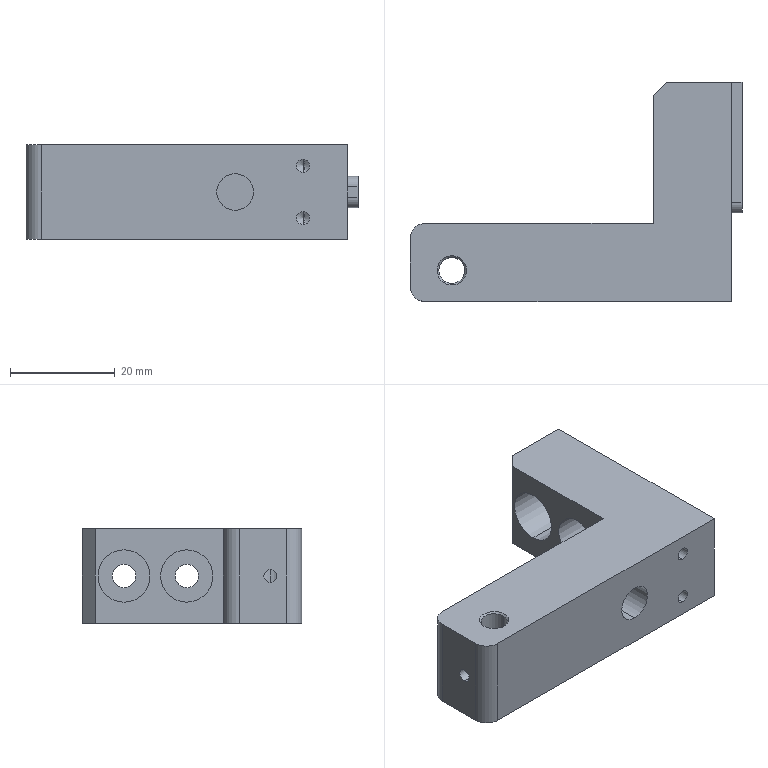Part | NX | features BREP 1 | 1 solid | 54 faces | box 63.5 x 42 x 18 mm | volume 21404 mm3 | cylinder 26 | plane 16 | cone 12 | commonest cylinder face diameters 2.5 x6 3.3 x4 4.5 x4 10 x4 4 x2 5 x2
STEP:
#1=CARTESIAN_POINT('',(0.,17.,-1.));
#2=VERTEX_POINT('',#1);
#3=CARTESIAN_POINT('',(0.,19.,-3.));
#4=VERTEX_POINT('',#3);
#5=CARTESIAN_POINT('',(0.,19.,-1.));
#6=DIRECTION('',(1.,0.,0.));
#7=DIRECTION('',(0.,0.,1.));
#8=AXIS2_PLACEMENT_3D('',#5,#6,#7);
#9=CIRCLE('',#8,2.);
#10=EDGE_CURVE('',#2,#4,#9,.T.);
#11=ORIENTED_EDGE('',*,*,#10,.T.);
#12=CARTESIAN_POINT('',(2.,19.,-3.));
#13=VERTEX_POINT('',#12);
#14=CARTESIAN_POINT('',(2.,19.,-3.));
#15=DIRECTION('',(-1.,0.,0.));
#16=VECTOR('',#15,1000.);
#17=LINE('',#14,#16);
#18=EDGE_CURVE('',#13,#4,#17,.T.);
#19=ORIENTED_EDGE('',*,*,#18,.F.);
#20=CARTESIAN_POINT('',(2.,17.,-1.));
#21=VERTEX_POINT('',#20);
#22=CARTESIAN_POINT('',(2.,19.,-1.));
#23=DIRECTION('',(1.,0.,0.));
#24=DIRECTION('',(0.,0.,1.));
#25=AXIS2_PLACEMENT_3D('',#22,#23,#24);
#26=CIRCLE('',#25,2.);
#27=EDGE_CURVE('',#21,#13,#26,.T.);
#28=ORIENTED_EDGE('',*,*,#27,.F.);
#29=CARTESIAN_POINT('',(2.,17.,-1.));
#30=DIRECTION('',(-1.,0.,0.));
#31=VECTOR('',#30,1000.);
#32=LINE('',#29,#31);
#33=EDGE_CURVE('',#21,#2,#32,.T.);
#34=ORIENTED_EDGE('',*,*,#33,.T.);
#35=EDGE_LOOP('',(#11,#19,#28,#34));
#36=FACE_BOUND('',#35,.T.);
#37=CARTESIAN_POINT('',(2.,19.,-1.));
#38=DIRECTION('',(-1.,0.,0.));
#39=DIRECTION('',(0.,0.,1.));
#40=AXIS2_PLACEMENT_3D('',#37,#38,#39);
#41=CYLINDRICAL_SURFACE('',#40,2.);
#42=ADVANCED_FACE('',(#36),#41,.T.);
#43=CARTESIAN_POINT('',(0.,17.,1.));
#44=VERTEX_POINT('',#43);
#45=CARTESIAN_POINT('',(0.,17.,1.));
#46=DIRECTION('',(0.,0.,-1.));
#47=VECTOR('',#46,1000.);
#48=LINE('',#45,#47);
#49=EDGE_CURVE('',#44,#2,#48,.T.);
#50=ORIENTED_EDGE('',*,*,#49,.T.);
#51=ORIENTED_EDGE('',*,*,#33,.F.);
#52=CARTESIAN_POINT('',(2.,17.,1.));
#53=VERTEX_POINT('',#52);
#54=CARTESIAN_POINT('',(2.,17.,1.));
#55=DIRECTION('',(0.,0.,-1.));
#56=VECTOR('',#55,1000.);
#57=LINE('',#54,#56);
#58=EDGE_CURVE('',#53,#21,#57,.T.);
#59=ORIENTED_EDGE('',*,*,#58,.F.);
#60=CARTESIAN_POINT('',(2.,17.,1.));
#61=DIRECTION('',(-1.,0.,0.));
#62=VECTOR('',#61,1000.);
#63=LINE('',#60,#62);
#64=EDGE_CURVE('',#53,#44,#63,.T.);
#65=ORIENTED_EDGE('',*,*,#64,.T.);
#66=EDGE_LOOP('',(#50,#51,#59,#65));
#67=FACE_BOUND('',#66,.T.);
#68=CARTESIAN_POINT('',(2.,17.,1.));
#69=DIRECTION('',(0.,1.,0.));
#70=DIRECTION('',(0.,0.,1.));
#71=AXIS2_PLACEMENT_3D('',#68,#69,#70);
#72=PLANE('',#71);
#73=ADVANCED_FACE('',(#67),#72,.F.);
#74=CARTESIAN_POINT('',(0.,19.,3.));
#75=VERTEX_POINT('',#74);
#76=CARTESIAN_POINT('',(0.,19.,1.));
#77=DIRECTION('',(1.,0.,0.));
#78=DIRECTION('',(0.,0.,1.));
#79=AXIS2_PLACEMENT_3D('',#76,#77,#78);
#80=CIRCLE('',#79,2.);
#81=EDGE_CURVE('',#75,#44,#80,.T.);
#82=ORIENTED_EDGE('',*,*,#81,.T.);
#83=ORIENTED_EDGE('',*,*,#64,.F.);
#84=CARTESIAN_POINT('',(2.,19.,3.));
#85=VERTEX_POINT('',#84);
#86=CARTESIAN_POINT('',(2.,19.,1.));
#87=DIRECTION('',(1.,0.,0.));
#88=DIRECTION('',(0.,0.,1.));
#89=AXIS2_PLACEMENT_3D('',#86,#87,#88);
#90=CIRCLE('',#89,2.);
#91=EDGE_CURVE('',#85,#53,#90,.T.);
#92=ORIENTED_EDGE('',*,*,#91,.F.);
#93=CARTESIAN_POINT('',(2.,19.,3.));
#94=DIRECTION('',(-1.,0.,0.));
#95=VECTOR('',#94,1000.);
#96=LINE('',#93,#95);
#97=EDGE_CURVE('',#85,#75,#96,.T.);
#98=ORIENTED_EDGE('',*,*,#97,.T.);
#99=EDGE_LOOP('',(#82,#83,#92,#98));
#100=FACE_BOUND('',#99,.T.);
#101=CARTESIAN_POINT('',(2.,19.,1.));
#102=DIRECTION('',(-1.,0.,0.));
#103=DIRECTION('',(0.,0.,1.));
#104=AXIS2_PLACEMENT_3D('',#101,#102,#103);
#105=CYLINDRICAL_SURFACE('',#104,2.);
#106=ADVANCED_FACE('',(#100),#105,.T.);
#107=CARTESIAN_POINT('',(0.,42.,3.));
#108=VERTEX_POINT('',#107);
#109=CARTESIAN_POINT('',(0.,19.,3.));
#110=DIRECTION('',(0.,-1.,0.));
#111=VECTOR('',#110,1000.);
#112=LINE('',#109,#111);
#113=EDGE_CURVE('',#108,#75,#112,.T.);
#114=ORIENTED_EDGE('',*,*,#113,.T.);
#115=ORIENTED_EDGE('',*,*,#97,.F.);
#116=CARTESIAN_POINT('',(2.,42.,3.));
#117=VERTEX_POINT('',#116);
#118=CARTESIAN_POINT('',(2.,19.,3.));
#119=DIRECTION('',(0.,-1.,0.));
#120=VECTOR('',#119,1000.);
#121=LINE('',#118,#120);
#122=EDGE_CURVE('',#117,#85,#121,.T.);
#123=ORIENTED_EDGE('',*,*,#122,.F.);
#124=CARTESIAN_POINT('',(2.,42.,3.));
#125=DIRECTION('',(-1.,0.,0.));
#126=VECTOR('',#125,1000.);
#127=LINE('',#124,#126);
#128=EDGE_CURVE('',#117,#108,#127,.T.);
#129=ORIENTED_EDGE('',*,*,#128,.T.);
#130=EDGE_LOOP('',(#114,#115,#123,#129));
#131=FACE_BOUND('',#130,.T.);
#132=CARTESIAN_POINT('',(2.,19.,3.));
#133=DIRECTION('',(0.,0.,-1.));
#134=DIRECTION('',(-1.,0.,0.));
#135=AXIS2_PLACEMENT_3D('',#132,#133,#134);
#136=PLANE('',#135);
#137=ADVANCED_FACE('',(#131),#136,.F.);
#138=CARTESIAN_POINT('',(0.,42.,-3.));
#139=VERTEX_POINT('',#138);
#140=CARTESIAN_POINT('',(0.,19.,-3.));
#141=DIRECTION('',(0.,1.,0.));
#142=VECTOR('',#141,1000.);
#143=LINE('',#140,#142);
#144=EDGE_CURVE('',#4,#139,#143,.T.);
#145=ORIENTED_EDGE('',*,*,#144,.T.);
#146=CARTESIAN_POINT('',(2.,42.,-3.));
#147=VERTEX_POINT('',#146);
#148=CARTESIAN_POINT('',(2.,42.,-3.));
#149=DIRECTION('',(-1.,0.,0.));
#150=VECTOR('',#149,1000.);
#151=LINE('',#148,#150);
#152=EDGE_CURVE('',#147,#139,#151,.T.);
#153=ORIENTED_EDGE('',*,*,#152,.F.);
#154=CARTESIAN_POINT('',(2.,19.,-3.));
#155=DIRECTION('',(0.,1.,0.));
#156=VECTOR('',#155,1000.);
#157=LINE('',#154,#156);
#158=EDGE_CURVE('',#13,#147,#157,.T.);
#159=ORIENTED_EDGE('',*,*,#158,.F.);
#160=ORIENTED_EDGE('',*,*,#18,.T.);
#161=EDGE_LOOP('',(#145,#153,#159,#160));
#162=FACE_BOUND('',#161,.T.);
#163=CARTESIAN_POINT('',(2.,19.,-3.));
#164=DIRECTION('',(0.,0.,1.));
#165=DIRECTION('',(1.,0.,0.));
#166=AXIS2_PLACEMENT_3D('',#163,#164,#165);
#167=PLANE('',#166);
#168=ADVANCED_FACE('',(#162),#167,.F.);
#169=CARTESIAN_POINT('',(2.,34.,2.25));
#170=VERTEX_POINT('',#169);
#171=CARTESIAN_POINT('',(2.,34.,-2.25));
#172=VERTEX_POINT('',#171);
#173=CARTESIAN_POINT('',(2.,34.,0.));
#174=DIRECTION('',(1.,0.,0.));
#175=DIRECTION('',(0.,0.,-1.));
#176=AXIS2_PLACEMENT_3D('',#173,#174,#175);
#177=CIRCLE('',#176,2.25);
#178=EDGE_CURVE('',#170,#172,#177,.T.);
#179=ORIENTED_EDGE('',*,*,#178,.F.);
#180=CARTESIAN_POINT('',(2.,34.,0.));
#181=DIRECTION('',(1.,0.,0.));
#182=DIRECTION('',(0.,0.,-1.));
#183=AXIS2_PLACEMENT_3D('',#180,#181,#182);
#184=CIRCLE('',#183,2.25);
#185=EDGE_CURVE('',#172,#170,#184,.T.);
#186=ORIENTED_EDGE('',*,*,#185,.F.);
#187=EDGE_LOOP('',(#179,#186));
#188=FACE_BOUND('',#187,.T.);
#189=CARTESIAN_POINT('',(2.,22.,2.25));
#190=VERTEX_POINT('',#189);
#191=CARTESIAN_POINT('',(2.,22.,-2.25));
#192=VERTEX_POINT('',#191);
#193=CARTESIAN_POINT('',(2.,22.,0.));
#194=DIRECTION('',(1.,0.,0.));
#195=DIRECTION('',(0.,0.,-1.));
#196=AXIS2_PLACEMENT_3D('',#193,#194,#195);
#197=CIRCLE('',#196,2.25);
#198=EDGE_CURVE('',#190,#192,#197,.T.);
#199=ORIENTED_EDGE('',*,*,#198,.F.);
#200=CARTESIAN_POINT('',(2.,22.,0.));
#201=DIRECTION('',(1.,0.,0.));
#202=DIRECTION('',(0.,0.,-1.));
#203=AXIS2_PLACEMENT_3D('',#200,#201,#202);
#204=CIRCLE('',#203,2.25);
#205=EDGE_CURVE('',#192,#190,#204,.T.);
#206=ORIENTED_EDGE('',*,*,#205,.F.);
#207=EDGE_LOOP('',(#199,#206));
#208=FACE_BOUND('',#207,.T.);
#209=ORIENTED_EDGE('',*,*,#158,.T.);
#210=CARTESIAN_POINT('',(2.,42.,3.));
#211=DIRECTION('',(0.,0.,1.));
#212=VECTOR('',#211,1000.);
#213=LINE('',#210,#212);
#214=EDGE_CURVE('',#147,#117,#213,.T.);
#215=ORIENTED_EDGE('',*,*,#214,.T.);
#216=ORIENTED_EDGE('',*,*,#122,.T.);
#217=ORIENTED_EDGE('',*,*,#91,.T.);
#218=ORIENTED_EDGE('',*,*,#58,.T.);
#219=ORIENTED_EDGE('',*,*,#27,.T.);
#220=EDGE_LOOP('',(#209,#215,#216,#217,#218,#219));
#221=FACE_BOUND('',#220,.T.);
#222=CARTESIAN_POINT('',(2.,19.,1.));
#223=DIRECTION('',(-1.,0.,0.));
#224=DIRECTION('',(0.,0.,1.));
#225=AXIS2_PLACEMENT_3D('',#222,#223,#224);
#226=PLANE('',#225);
#227=ADVANCED_FACE('',(#188,#208,#221),#226,.F.);
#228=CARTESIAN_POINT('',(-49.,15.,-1.65));
#229=VERTEX_POINT('',#228);
#230=CARTESIAN_POINT('',(-49.,4.9,-1.65));
#231=VERTEX_POINT('',#230);
#232=CARTESIAN_POINT('',(-49.,15.,-1.65));
#233=DIRECTION('',(0.,1.,0.));
#234=VECTOR('',#233,1000.);
#235=LINE('',#232,#234);
#236=EDGE_CURVE('',#229,#231,#235,.F.);
#237=ORIENTED_EDGE('',*,*,#236,.T.);
#238=CARTESIAN_POINT('',(-49.,4.9,1.65));
#239=VERTEX_POINT('',#238);
#240=CARTESIAN_POINT('',(-49.,4.9,0.));
#241=DIRECTION('',(0.,1.,0.));
#242=DIRECTION('',(0.,0.,1.));
#243=AXIS2_PLACEMENT_3D('',#240,#241,#242);
#244=CIRCLE('',#243,1.65);
#245=EDGE_CURVE('',#239,#231,#244,.T.);
#246=ORIENTED_EDGE('',*,*,#245,.F.);
#247=CARTESIAN_POINT('',(-49.,15.,1.65));
#248=VERTEX_POINT('',#247);
#249=CARTESIAN_POINT('',(-49.,15.,1.65));
#250=DIRECTION('',(0.,1.,0.));
#251=VECTOR('',#250,1000.);
#252=LINE('',#249,#251);
#253=EDGE_CURVE('',#248,#239,#252,.F.);
#254=ORIENTED_EDGE('',*,*,#253,.F.);
#255=CARTESIAN_POINT('',(-49.,15.,0.));
#256=DIRECTION('',(0.,1.,0.));
#257=DIRECTION('',(0.,0.,1.));
#258=AXIS2_PLACEMENT_3D('',#255,#256,#257);
#259=CIRCLE('',#258,1.65);
#260=EDGE_CURVE('',#248,#229,#259,.T.);
#261=ORIENTED_EDGE('',*,*,#260,.T.);
#262=EDGE_LOOP('',(#237,#246,#254,#261));
#263=FACE_BOUND('',#262,.T.);
#264=CARTESIAN_POINT('',(-49.,15.,0.));
#265=DIRECTION('',(0.,1.,0.));
#266=DIRECTION('',(0.,0.,1.));
#267=AXIS2_PLACEMENT_3D('',#264,#265,#266);
#268=CYLINDRICAL_SURFACE('',#267,1.65);
#269=ADVANCED_FACE('',(#263),#268,.F.);
#270=CARTESIAN_POINT('',(-49.,3.909,0.));
#271=VERTEX_POINT('',#270);
#272=CARTESIAN_POINT('',(-49.,4.9,-1.65));
#273=DIRECTION('',(0.,0.515,-0.8572));
#274=VECTOR('',#273,1000.);
#275=LINE('',#272,#274);
#276=EDGE_CURVE('',#271,#231,#275,.T.);
#277=ORIENTED_EDGE('',*,*,#276,.F.);
#278=CARTESIAN_POINT('',(-49.,4.9,1.65));
#279=DIRECTION('',(0.,0.515,0.8572));
#280=VECTOR('',#279,1000.);
#281=LINE('',#278,#280);
#282=EDGE_CURVE('',#271,#239,#281,.T.);
#283=ORIENTED_EDGE('',*,*,#282,.T.);
#284=ORIENTED_EDGE('',*,*,#245,.T.);
#285=EDGE_LOOP('',(#277,#283,#284));
#286=FACE_BOUND('',#285,.T.);
#287=CARTESIAN_POINT('',(-49.,4.9,0.));
#288=DIRECTION('',(0.,1.,0.));
#289=DIRECTION('',(0.,0.,1.));
#290=AXIS2_PLACEMENT_3D('',#287,#288,#289);
#291=CONICAL_SURFACE('',#290,1.65,1.03);
#292=ADVANCED_FACE('',(#286),#291,.F.);
#293=CARTESIAN_POINT('',(-35.,15.,-1.65));
#294=VERTEX_POINT('',#293);
#295=CARTESIAN_POINT('',(-35.,4.9,-1.65));
#296=VERTEX_POINT('',#295);
#297=CARTESIAN_POINT('',(-35.,15.,-1.65));
#298=DIRECTION('',(0.,1.,0.));
#299=VECTOR('',#298,1000.);
#300=LINE('',#297,#299);
#301=EDGE_CURVE('',#294,#296,#300,.F.);
#302=ORIENTED_EDGE('',*,*,#301,.T.);
#303=CARTESIAN_POINT('',(-35.,4.9,1.65));
#304=VERTEX_POINT('',#303);
#305=CARTESIAN_POINT('',(-35.,4.9,0.));
#306=DIRECTION('',(0.,1.,0.));
#307=DIRECTION('',(0.,0.,1.));
#308=AXIS2_PLACEMENT_3D('',#305,#306,#307);
#309=CIRCLE('',#308,1.65);
#310=EDGE_CURVE('',#304,#296,#309,.T.);
#311=ORIENTED_EDGE('',*,*,#310,.F.);
#312=CARTESIAN_POINT('',(-35.,15.,1.65));
#313=VERTEX_POINT('',#312);
#314=CARTESIAN_POINT('',(-35.,15.,1.65));
#315=DIRECTION('',(0.,1.,0.));
#316=VECTOR('',#315,1000.);
#317=LINE('',#314,#316);
#318=EDGE_CURVE('',#313,#304,#317,.F.);
#319=ORIENTED_EDGE('',*,*,#318,.F.);
#320=CARTESIAN_POINT('',(-35.,15.,0.));
#321=DIRECTION('',(0.,1.,0.));
#322=DIRECTION('',(0.,0.,1.));
#323=AXIS2_PLACEMENT_3D('',#320,#321,#322);
#324=CIRCLE('',#323,1.65);
#325=EDGE_CURVE('',#313,#294,#324,.T.);
#326=ORIENTED_EDGE('',*,*,#325,.T.);
#327=EDGE_LOOP('',(#302,#311,#319,#326));
#328=FACE_BOUND('',#327,.T.);
#329=CARTESIAN_POINT('',(-35.,15.,0.));
#330=DIRECTION('',(0.,1.,0.));
#331=DIRECTION('',(0.,0.,1.));
#332=AXIS2_PLACEMENT_3D('',#329,#330,#331);
#333=CYLINDRICAL_SURFACE('',#332,1.65);
#334=ADVANCED_FACE('',(#328),#333,.F.);
#335=CARTESIAN_POINT('',(-35.,3.909,0.));
#336=VERTEX_POINT('',#335);
#337=CARTESIAN_POINT('',(-35.,4.9,-1.65));
#338=DIRECTION('',(0.,0.515,-0.8572));
#339=VECTOR('',#338,1000.);
#340=LINE('',#337,#339);
#341=EDGE_CURVE('',#336,#296,#340,.T.);
#342=ORIENTED_EDGE('',*,*,#341,.F.);
#343=CARTESIAN_POINT('',(-35.,4.9,1.65));
#344=DIRECTION('',(0.,0.515,0.8572));
#345=VECTOR('',#344,1000.);
#346=LINE('',#343,#345);
#347=EDGE_CURVE('',#336,#304,#346,.T.);
#348=ORIENTED_EDGE('',*,*,#347,.T.);
#349=ORIENTED_EDGE('',*,*,#310,.T.);
#350=EDGE_LOOP('',(#342,#348,#349));
#351=FACE_BOUND('',#350,.T.);
#352=CARTESIAN_POINT('',(-35.,4.9,0.));
#353=DIRECTION('',(0.,1.,0.));
#354=DIRECTION('',(0.,0.,1.));
#355=AXIS2_PLACEMENT_3D('',#352,#353,#354);
#356=CONICAL_SURFACE('',#355,1.65,1.03);
#357=ADVANCED_FACE('',(#351),#356,.F.);
#358=CARTESIAN_POINT('',(-8.5,9.5,6.25));
#359=VERTEX_POINT('',#358);
#360=CARTESIAN_POINT('',(-8.5,0.,6.25));
#361=VERTEX_POINT('',#360);
#362=CARTESIAN_POINT('',(-8.5,0.,6.25));
#363=DIRECTION('',(0.,-1.,0.));
#364=VECTOR('',#363,1000.);
#365=LINE('',#362,#364);
#366=EDGE_CURVE('',#359,#361,#365,.T.);
#367=ORIENTED_EDGE('',*,*,#366,.F.);
#368=CARTESIAN_POINT('',(-8.5,9.5,3.75));
#369=VERTEX_POINT('',#368);
#370=CARTESIAN_POINT('',(-8.5,9.5,5.));
#371=DIRECTION('',(0.,-1.,0.));
#372=DIRECTION('',(0.,0.,-1.));
#373=AXIS2_PLACEMENT_3D('',#370,#371,#372);
#374=CIRCLE('',#373,1.25);
#375=EDGE_CURVE('',#369,#359,#374,.T.);
#376=ORIENTED_EDGE('',*,*,#375,.F.);
#377=CARTESIAN_POINT('',(-8.5,0.,3.75));
#378=VERTEX_POINT('',#377);
#379=CARTESIAN_POINT('',(-8.5,0.,3.75));
#380=DIRECTION('',(0.,-1.,0.));
#381=VECTOR('',#380,1000.);
#382=LINE('',#379,#381);
#383=EDGE_CURVE('',#369,#378,#382,.T.);
#384=ORIENTED_EDGE('',*,*,#383,.T.);
#385=CARTESIAN_POINT('',(-8.5,0.,5.));
#386=DIRECTION('',(0.,-1.,0.));
#387=DIRECTION('',(0.,0.,-1.));
#388=AXIS2_PLACEMENT_3D('',#385,#386,#387);
#389=CIRCLE('',#388,1.25);
#390=EDGE_CURVE('',#378,#361,#389,.T.);
#391=ORIENTED_EDGE('',*,*,#390,.T.);
#392=EDGE_LOOP('',(#367,#376,#384,#391));
#393=FACE_BOUND('',#392,.T.);
#394=CARTESIAN_POINT('',(-8.5,0.,5.));
#395=DIRECTION('',(0.,-1.,0.));
#396=DIRECTION('',(0.,0.,-1.));
#397=AXIS2_PLACEMENT_3D('',#394,#395,#396);
#398=CYLINDRICAL_SURFACE('',#397,1.25);
#399=ADVANCED_FACE('',(#393),#398,.F.);
#400=CARTESIAN_POINT('',(-8.5,10.251,5.));
#401=VERTEX_POINT('',#400);
#402=CARTESIAN_POINT('',(-8.5,9.5,6.25));
#403=DIRECTION('',(0.,-0.515,0.8572));
#404=VECTOR('',#403,1000.);
#405=LINE('',#402,#404);
#406=EDGE_CURVE('',#359,#401,#405,.F.);
#407=ORIENTED_EDGE('',*,*,#406,.T.);
#408=CARTESIAN_POINT('',(-8.5,9.5,3.75));
#409=DIRECTION('',(0.,-0.515,-0.8572));
#410=VECTOR('',#409,1000.);
#411=LINE('',#408,#410);
#412=EDGE_CURVE('',#369,#401,#411,.F.);
#413=ORIENTED_EDGE('',*,*,#412,.F.);
#414=ORIENTED_EDGE('',*,*,#375,.T.);
#415=EDGE_LOOP('',(#407,#413,#414));
#416=FACE_BOUND('',#415,.T.);
#417=CARTESIAN_POINT('',(-8.5,9.5,5.));
#418=DIRECTION('',(0.,-1.,0.));
#419=DIRECTION('',(0.,0.,-1.));
#420=AXIS2_PLACEMENT_3D('',#417,#418,#419);
#421=CONICAL_SURFACE('',#420,1.25,1.03);
#422=ADVANCED_FACE('',(#416),#421,.F.);
#423=CARTESIAN_POINT('',(-8.5,9.5,-3.75));
#424=VERTEX_POINT('',#423);
#425=CARTESIAN_POINT('',(-8.5,0.,-3.75));
#426=VERTEX_POINT('',#425);
#427=CARTESIAN_POINT('',(-8.5,0.,-3.75));
#428=DIRECTION('',(0.,-1.,0.));
#429=VECTOR('',#428,1000.);
#430=LINE('',#427,#429);
#431=EDGE_CURVE('',#424,#426,#430,.T.);
#432=ORIENTED_EDGE('',*,*,#431,.F.);
#433=CARTESIAN_POINT('',(-8.5,9.5,-6.25));
#434=VERTEX_POINT('',#433);
#435=CARTESIAN_POINT('',(-8.5,9.5,-5.));
#436=DIRECTION('',(0.,-1.,0.));
#437=DIRECTION('',(0.,0.,-1.));
#438=AXIS2_PLACEMENT_3D('',#435,#436,#437);
#439=CIRCLE('',#438,1.25);
#440=EDGE_CURVE('',#434,#424,#439,.T.);
#441=ORIENTED_EDGE('',*,*,#440,.F.);
#442=CARTESIAN_POINT('',(-8.5,0.,-6.25));
#443=VERTEX_POINT('',#442);
#444=CARTESIAN_POINT('',(-8.5,0.,-6.25));
#445=DIRECTION('',(0.,-1.,0.));
#446=VECTOR('',#445,1000.);
#447=LINE('',#444,#446);
#448=EDGE_CURVE('',#434,#443,#447,.T.);
#449=ORIENTED_EDGE('',*,*,#448,.T.);
#450=CARTESIAN_POINT('',(-8.5,0.,-5.));
#451=DIRECTION('',(0.,-1.,0.));
#452=DIRECTION('',(0.,0.,-1.));
#453=AXIS2_PLACEMENT_3D('',#450,#451,#452);
#454=CIRCLE('',#453,1.25);
#455=EDGE_CURVE('',#443,#426,#454,.T.);
#456=ORIENTED_EDGE('',*,*,#455,.T.);
#457=EDGE_LOOP('',(#432,#441,#449,#456));
#458=FACE_BOUND('',#457,.T.);
#459=CARTESIAN_POINT('',(-8.5,0.,-5.));
#460=DIRECTION('',(0.,-1.,0.));
#461=DIRECTION('',(0.,0.,-1.));
#462=AXIS2_PLACEMENT_3D('',#459,#460,#461);
#463=CYLINDRICAL_SURFACE('',#462,1.25);
#464=ADVANCED_FACE('',(#458),#463,.F.);
#465=CARTESIAN_POINT('',(-8.5,10.251,-5.));
#466=VERTEX_POINT('',#465);
#467=CARTESIAN_POINT('',(-8.5,9.5,-3.75));
#468=DIRECTION('',(0.,-0.515,0.8572));
#469=VECTOR('',#468,1000.);
#470=LINE('',#467,#469);
#471=EDGE_CURVE('',#424,#466,#470,.F.);
#472=ORIENTED_EDGE('',*,*,#471,.T.);
#473=CARTESIAN_POINT('',(-8.5,9.5,-6.25));
#474=DIRECTION('',(0.,-0.515,-0.8572));
#475=VECTOR('',#474,1000.);
#476=LINE('',#473,#475);
#477=EDGE_CURVE('',#434,#466,#476,.F.);
#478=ORIENTED_EDGE('',*,*,#477,.F.);
#479=ORIENTED_EDGE('',*,*,#440,.T.);
#480=EDGE_LOOP('',(#472,#478,#479));
#481=FACE_BOUND('',#480,.T.);
#482=CARTESIAN_POINT('',(-8.5,9.5,-5.));
#483=DIRECTION('',(0.,-1.,0.));
#484=DIRECTION('',(0.,0.,-1.));
#485=AXIS2_PLACEMENT_3D('',#482,#483,#484);
#486=CONICAL_SURFACE('',#485,1.25,1.03);
#487=ADVANCED_FACE('',(#481),#486,.F.);
#488=CARTESIAN_POINT('',(-51.,6.,-8.7));
#489=VERTEX_POINT('',#488);
#490=CARTESIAN_POINT('',(-50.7,6.,-9.));
#491=VERTEX_POINT('',#490);
#492=CARTESIAN_POINT('',(-50.7,6.,-9.));
#493=DIRECTION('',(0.7071,0.,-0.7071));
#494=VECTOR('',#493,1000.);
#495=LINE('',#492,#494);
#496=EDGE_CURVE('',#489,#491,#495,.T.);
#497=ORIENTED_EDGE('',*,*,#496,.F.);
#498=CARTESIAN_POINT('',(-56.,6.,-8.7));
#499=VERTEX_POINT('',#498);
#500=CARTESIAN_POINT('',(-53.5,6.,-8.7));
#501=DIRECTION('',(0.,0.,-1.));
#502=DIRECTION('',(1.,0.,0.));
#503=AXIS2_PLACEMENT_3D('',#500,#501,#502);
#504=CIRCLE('',#503,2.5);
#505=EDGE_CURVE('',#499,#489,#504,.T.);
#506=ORIENTED_EDGE('',*,*,#505,.F.);
#507=CARTESIAN_POINT('',(-56.3,6.,-9.));
#508=VERTEX_POINT('',#507);
#509=CARTESIAN_POINT('',(-56.3,6.,-9.));
#510=DIRECTION('',(-0.7071,0.,-0.7071));
#511=VECTOR('',#510,1000.);
#512=LINE('',#509,#511);
#513=EDGE_CURVE('',#499,#508,#512,.T.);
#514=ORIENTED_EDGE('',*,*,#513,.T.);
#515=CARTESIAN_POINT('',(-53.5,6.,-9.));
#516=DIRECTION('',(0.,0.,1.));
#517=DIRECTION('',(1.,0.,0.));
#518=AXIS2_PLACEMENT_3D('',#515,#516,#517);
#519=CIRCLE('',#518,2.8);
#520=EDGE_CURVE('',#491,#508,#519,.T.);
#521=ORIENTED_EDGE('',*,*,#520,.F.);
#522=EDGE_LOOP('',(#497,#506,#514,#521));
#523=FACE_BOUND('',#522,.T.);
#524=CARTESIAN_POINT('',(-53.5,6.,-9.));
#525=DIRECTION('',(0.,0.,-1.));
#526=DIRECTION('',(-1.,0.,0.));
#527=AXIS2_PLACEMENT_3D('',#524,#525,#526);
#528=CONICAL_SURFACE('',#527,2.8,0.7854);
#529=ADVANCED_FACE('',(#523),#528,.F.);
#530=CARTESIAN_POINT('',(-56.3,6.,9.));
#531=VERTEX_POINT('',#530);
#532=CARTESIAN_POINT('',(-56.,6.,8.7));
#533=VERTEX_POINT('',#532);
#534=CARTESIAN_POINT('',(-56.,6.,8.7));
#535=DIRECTION('',(-0.7071,0.,0.7071));
#536=VECTOR('',#535,1000.);
#537=LINE('',#534,#536);
#538=EDGE_CURVE('',#531,#533,#537,.F.);
#539=ORIENTED_EDGE('',*,*,#538,.T.);
#540=CARTESIAN_POINT('',(-51.,6.,8.7));
#541=VERTEX_POINT('',#540);
#542=CARTESIAN_POINT('',(-53.5,6.,8.7));
#543=DIRECTION('',(0.,0.,1.));
#544=DIRECTION('',(1.,0.,0.));
#545=AXIS2_PLACEMENT_3D('',#542,#543,#544);
#546=CIRCLE('',#545,2.5);
#547=EDGE_CURVE('',#541,#533,#546,.T.);
#548=ORIENTED_EDGE('',*,*,#547,.F.);
#549=CARTESIAN_POINT('',(-50.7,6.,9.));
#550=VERTEX_POINT('',#549);
#551=CARTESIAN_POINT('',(-51.,6.,8.7));
#552=DIRECTION('',(0.7071,0.,0.7071));
#553=VECTOR('',#552,1000.);
#554=LINE('',#551,#553);
#555=EDGE_CURVE('',#550,#541,#554,.F.);
#556=ORIENTED_EDGE('',*,*,#555,.F.);
#557=CARTESIAN_POINT('',(-53.5,6.,9.));
#558=DIRECTION('',(0.,0.,-1.));
#559=DIRECTION('',(1.,0.,0.));
#560=AXIS2_PLACEMENT_3D('',#557,#558,#559);
#561=CIRCLE('',#560,2.8);
#562=EDGE_CURVE('',#531,#550,#561,.T.);
#563=ORIENTED_EDGE('',*,*,#562,.F.);
#564=EDGE_LOOP('',(#539,#548,#556,#563));
#565=FACE_BOUND('',#564,.T.);
#566=CARTESIAN_POINT('',(-53.5,6.,8.7));
#567=DIRECTION('',(0.,0.,1.));
#568=DIRECTION('',(1.,0.,0.));
#569=AXIS2_PLACEMENT_3D('',#566,#567,#568);
#570=CONICAL_SURFACE('',#569,2.5,0.7854);
#571=ADVANCED_FACE('',(#565),#570,.F.);
#572=CARTESIAN_POINT('',(-61.5,6.,-1.25));
#573=VERTEX_POINT('',#572);
#574=CARTESIAN_POINT('',(-56.,6.,-1.25));
#575=VERTEX_POINT('',#574);
#576=CARTESIAN_POINT('',(-61.5,6.,-1.25));
#577=DIRECTION('',(-1.,0.,0.));
#578=VECTOR('',#577,1000.);
#579=LINE('',#576,#578);
#580=EDGE_CURVE('',#573,#575,#579,.F.);
#581=ORIENTED_EDGE('',*,*,#580,.T.);
#582=CARTESIAN_POINT('',(-56.,6.,1.25));
#583=VERTEX_POINT('',#582);
#584=CARTESIAN_POINT('',(-56.,6.,-1.25));
#585=CARTESIAN_POINT('',(-56.,6.158,-1.25));
#586=CARTESIAN_POINT('',(-55.968,6.441,-1.185));
#587=CARTESIAN_POINT('',(-55.912,6.662,-1.066));
#588=CARTESIAN_POINT('',(-55.856,6.845,-0.9353));
#589=CARTESIAN_POINT('',(-55.792,6.999,-0.7546));
#590=CARTESIAN_POINT('',(-55.772,7.044,-0.69));
#591=CARTESIAN_POINT('',(-55.69,7.213,-0.3989));
#592=CARTESIAN_POINT('',(-55.648,7.275,0.001591));
#593=CARTESIAN_POINT('',(-55.69,7.212,0.4001));
#594=CARTESIAN_POINT('',(-55.771,7.046,0.6879));
#595=CARTESIAN_POINT('',(-55.793,6.998,0.7553));
#596=CARTESIAN_POINT('',(-55.855,6.847,0.9334));
#597=CARTESIAN_POINT('',(-55.912,6.662,1.066));
#598=CARTESIAN_POINT('',(-55.968,6.442,1.185));
#599=CARTESIAN_POINT('',(-56.,6.158,1.25));
#600=CARTESIAN_POINT('',(-56.,6.,1.25));
#601=B_SPLINE_CURVE_WITH_KNOTS('',3,(#584,#585,#586,#587,#588,#589,#590,#591,#592,#593,#594,#595,#596,#597,#598,#599,#600),.UNSPECIFIED.,.F.,.F.,(4,1,1,1,1,1,1,1,1,1,1,1,1,1,4),(0.,0.125,0.1875,0.25,0.2812,0.3125,0.375,0.5,0.625,0.6875,0.7188,0.75,0.8125,0.875,1.),.UNSPECIFIED.);
#602=EDGE_CURVE('',#583,#575,#601,.F.);
#603=ORIENTED_EDGE('',*,*,#602,.F.);
#604=CARTESIAN_POINT('',(-61.5,6.,1.25));
#605=VERTEX_POINT('',#604);
#606=CARTESIAN_POINT('',(-61.5,6.,1.25));
#607=DIRECTION('',(-1.,0.,0.));
#608=VECTOR('',#607,1000.);
#609=LINE('',#606,#608);
#610=EDGE_CURVE('',#605,#583,#609,.F.);
#611=ORIENTED_EDGE('',*,*,#610,.F.);
#612=CARTESIAN_POINT('',(-61.5,6.,0.));
#613=DIRECTION('',(-1.,0.,0.));
#614=DIRECTION('',(0.,0.,1.));
#615=AXIS2_PLACEMENT_3D('',#612,#613,#614);
#616=CIRCLE('',#615,1.25);
#617=EDGE_CURVE('',#605,#573,#616,.T.);
#618=ORIENTED_EDGE('',*,*,#617,.T.);
#619=EDGE_LOOP('',(#581,#603,#611,#618));
#620=FACE_BOUND('',#619,.T.);
#621=CARTESIAN_POINT('',(-61.5,6.,0.));
#622=DIRECTION('',(-1.,0.,0.));
#623=DIRECTION('',(0.,0.,1.));
#624=AXIS2_PLACEMENT_3D('',#621,#622,#623);
#625=CYLINDRICAL_SURFACE('',#624,1.25);
#626=ADVANCED_FACE('',(#620),#625,.F.);
#627=CARTESIAN_POINT('',(-21.5,12.,-3.5));
#628=VERTEX_POINT('',#627);
#629=CARTESIAN_POINT('',(-21.5,12.,3.5));
#630=VERTEX_POINT('',#629);
#631=CARTESIAN_POINT('',(-21.5,12.,0.));
#632=DIRECTION('',(0.,-1.,0.));
#633=DIRECTION('',(0.,0.,-1.));
#634=AXIS2_PLACEMENT_3D('',#631,#632,#633);
#635=CIRCLE('',#634,3.5);
#636=EDGE_CURVE('',#628,#630,#635,.T.);
#637=ORIENTED_EDGE('',*,*,#636,.T.);
#638=CARTESIAN_POINT('',(-21.5,12.,0.));
#639=DIRECTION('',(0.,-1.,0.));
#640=DIRECTION('',(0.,0.,-1.));
#641=AXIS2_PLACEMENT_3D('',#638,#639,#640);
#642=CIRCLE('',#641,3.5);
#643=EDGE_CURVE('',#630,#628,#642,.T.);
#644=ORIENTED_EDGE('',*,*,#643,.T.);
#645=EDGE_LOOP('',(#637,#644));
#646=FACE_BOUND('',#645,.T.);
#647=CARTESIAN_POINT('',(-21.5,12.,0.));
#648=DIRECTION('',(0.,-1.,0.));
#649=DIRECTION('',(0.,0.,-1.));
#650=AXIS2_PLACEMENT_3D('',#647,#648,#649);
#651=PLANE('',#650);
#652=ADVANCED_FACE('',(#646),#651,.T.);
#653=CARTESIAN_POINT('',(-21.5,0.,3.5));
#654=VERTEX_POINT('',#653);
#655=CARTESIAN_POINT('',(-21.5,12.,3.5));
#656=DIRECTION('',(0.,-1.,0.));
#657=VECTOR('',#656,1000.);
#658=LINE('',#655,#657);
#659=EDGE_CURVE('',#630,#654,#658,.T.);
#660=ORIENTED_EDGE('',*,*,#659,.F.);
#661=ORIENTED_EDGE('',*,*,#636,.F.);
#662=CARTESIAN_POINT('',(-21.5,0.,-3.5));
#663=VERTEX_POINT('',#662);
#664=CARTESIAN_POINT('',(-21.5,12.,-3.5));
#665=DIRECTION('',(0.,-1.,0.));
#666=VECTOR('',#665,1000.);
#667=LINE('',#664,#666);
#668=EDGE_CURVE('',#628,#663,#667,.T.);
#669=ORIENTED_EDGE('',*,*,#668,.T.);
#670=CARTESIAN_POINT('',(-21.5,0.,0.));
#671=DIRECTION('',(0.,-1.,0.));
#672=DIRECTION('',(0.,0.,-1.));
#673=AXIS2_PLACEMENT_3D('',#670,#671,#672);
#674=CIRCLE('',#673,3.5);
#675=EDGE_CURVE('',#663,#654,#674,.T.);
#676=ORIENTED_EDGE('',*,*,#675,.T.);
#677=EDGE_LOOP('',(#660,#661,#669,#676));
#678=FACE_BOUND('',#677,.T.);
#679=CARTESIAN_POINT('',(-21.5,12.,0.));
#680=DIRECTION('',(0.,-1.,0.));
#681=DIRECTION('',(0.,0.,-1.));
#682=AXIS2_PLACEMENT_3D('',#679,#680,#681);
#683=CYLINDRICAL_SURFACE('',#682,3.5);
#684=ADVANCED_FACE('',(#678),#683,.F.);
#685=CARTESIAN_POINT('',(-58.5,15.,9.));
#686=VERTEX_POINT('',#685);
#687=CARTESIAN_POINT('',(-61.5,12.,9.));
#688=VERTEX_POINT('',#687);
#689=CARTESIAN_POINT('',(-58.5,12.,9.));
#690=DIRECTION('',(0.,0.,1.));
#691=DIRECTION('',(1.,0.,0.));
#692=AXIS2_PLACEMENT_3D('',#689,#690,#691);
#693=CIRCLE('',#692,3.);
#694=EDGE_CURVE('',#686,#688,#693,.T.);
#695=ORIENTED_EDGE('',*,*,#694,.F.);
#696=CARTESIAN_POINT('',(-58.5,15.,-9.));
#697=VERTEX_POINT('',#696);
#698=CARTESIAN_POINT('',(-58.5,15.,9.));
#699=DIRECTION('',(0.,0.,1.));
#700=VECTOR('',#699,1000.);
#701=LINE('',#698,#700);
#702=EDGE_CURVE('',#697,#686,#701,.T.);
#703=ORIENTED_EDGE('',*,*,#702,.F.);
#704=CARTESIAN_POINT('',(-61.5,12.,-9.));
#705=VERTEX_POINT('',#704);
#706=CARTESIAN_POINT('',(-58.5,12.,-9.));
#707=DIRECTION('',(0.,0.,-1.));
#708=DIRECTION('',(1.,0.,0.));
#709=AXIS2_PLACEMENT_3D('',#706,#707,#708);
#710=CIRCLE('',#709,3.);
#711=EDGE_CURVE('',#705,#697,#710,.T.);
#712=ORIENTED_EDGE('',*,*,#711,.F.);
#713=CARTESIAN_POINT('',(-61.5,12.,9.));
#714=DIRECTION('',(0.,0.,-1.));
#715=VECTOR('',#714,1000.);
#716=LINE('',#713,#715);
#717=EDGE_CURVE('',#688,#705,#716,.T.);
#718=ORIENTED_EDGE('',*,*,#717,.F.);
#719=EDGE_LOOP('',(#695,#703,#712,#718));
#720=FACE_BOUND('',#719,.T.);
#721=CARTESIAN_POINT('',(-58.5,12.,9.));
#722=DIRECTION('',(0.,0.,-1.));
#723=DIRECTION('',(-1.,0.,0.));
#724=AXIS2_PLACEMENT_3D('',#721,#722,#723);
#725=CYLINDRICAL_SURFACE('',#724,3.);
#726=ADVANCED_FACE('',(#720),#725,.T.);
#727=CARTESIAN_POINT('',(-61.5,3.,9.));
#728=VERTEX_POINT('',#727);
#729=CARTESIAN_POINT('',(-58.5,0.,9.));
#730=VERTEX_POINT('',#729);
#731=CARTESIAN_POINT('',(-58.5,3.,9.));
#732=DIRECTION('',(0.,0.,1.));
#733=DIRECTION('',(1.,0.,0.));
#734=AXIS2_PLACEMENT_3D('',#731,#732,#733);
#735=CIRCLE('',#734,3.);
#736=EDGE_CURVE('',#728,#730,#735,.T.);
#737=ORIENTED_EDGE('',*,*,#736,.F.);
#738=CARTESIAN_POINT('',(-61.5,3.,-9.));
#739=VERTEX_POINT('',#738);
#740=CARTESIAN_POINT('',(-61.5,3.,9.));
#741=DIRECTION('',(0.,0.,1.));
#742=VECTOR('',#741,1000.);
#743=LINE('',#740,#742);
#744=EDGE_CURVE('',#739,#728,#743,.T.);
#745=ORIENTED_EDGE('',*,*,#744,.F.);
#746=CARTESIAN_POINT('',(-58.5,0.,-9.));
#747=VERTEX_POINT('',#746);
#748=CARTESIAN_POINT('',(-58.5,3.,-9.));
#749=DIRECTION('',(0.,0.,-1.));
#750=DIRECTION('',(1.,0.,0.));
#751=AXIS2_PLACEMENT_3D('',#748,#749,#750);
#752=CIRCLE('',#751,3.);
#753=EDGE_CURVE('',#747,#739,#752,.T.);
#754=ORIENTED_EDGE('',*,*,#753,.F.);
#755=CARTESIAN_POINT('',(-58.5,0.,9.));
#756=DIRECTION('',(0.,0.,-1.));
#757=VECTOR('',#756,1000.);
#758=LINE('',#755,#757);
#759=EDGE_CURVE('',#730,#747,#758,.T.);
#760=ORIENTED_EDGE('',*,*,#759,.F.);
#761=EDGE_LOOP('',(#737,#745,#754,#760));
#762=FACE_BOUND('',#761,.T.);
#763=CARTESIAN_POINT('',(-58.5,3.,9.));
#764=DIRECTION('',(0.,0.,-1.));
#765=DIRECTION('',(-1.,0.,0.));
#766=AXIS2_PLACEMENT_3D('',#763,#764,#765);
#767=CYLINDRICAL_SURFACE('',#766,3.);
#768=ADVANCED_FACE('',(#762),#767,.T.);
#769=CARTESIAN_POINT('',(-56.,6.,9.));
#770=DIRECTION('',(0.,0.,1.));
#771=VECTOR('',#770,1000.);
#772=LINE('',#769,#771);
#773=EDGE_CURVE('',#575,#499,#772,.F.);
#774=ORIENTED_EDGE('',*,*,#773,.T.);
#775=ORIENTED_EDGE('',*,*,#505,.T.);
#776=CARTESIAN_POINT('',(-51.,6.,9.));
#777=DIRECTION('',(0.,0.,1.));
#778=VECTOR('',#777,1000.);
#779=LINE('',#776,#778);
#780=EDGE_CURVE('',#541,#489,#779,.F.);
#781=ORIENTED_EDGE('',*,*,#780,.F.);
#782=ORIENTED_EDGE('',*,*,#547,.T.);
#783=CARTESIAN_POINT('',(-56.,6.,9.));
#784=DIRECTION('',(0.,0.,1.));
#785=VECTOR('',#784,1000.);
#786=LINE('',#783,#785);
#787=EDGE_CURVE('',#583,#533,#786,.T.);
#788=ORIENTED_EDGE('',*,*,#787,.F.);
#789=ORIENTED_EDGE('',*,*,#602,.T.);
#790=EDGE_LOOP('',(#774,#775,#781,#782,#788,#789));
#791=FACE_BOUND('',#790,.T.);
#792=CARTESIAN_POINT('',(-53.5,6.,9.));
#793=DIRECTION('',(0.,0.,1.));
#794=DIRECTION('',(1.,0.,0.));
#795=AXIS2_PLACEMENT_3D('',#792,#793,#794);
#796=CYLINDRICAL_SURFACE('',#795,2.5);
#797=ADVANCED_FACE('',(#791),#796,.F.);
#798=CARTESIAN_POINT('',(-12.5,42.,9.));
#799=VERTEX_POINT('',#798);
#800=CARTESIAN_POINT('',(-15.,39.5,9.));
#801=VERTEX_POINT('',#800);
#802=CARTESIAN_POINT('',(-27.25,27.25,9.));
#803=DIRECTION('',(-0.7071,-0.7071,0.));
#804=VECTOR('',#803,1000.);
#805=LINE('',#802,#804);
#806=EDGE_CURVE('',#799,#801,#805,.T.);
#807=ORIENTED_EDGE('',*,*,#806,.F.);
#808=CARTESIAN_POINT('',(-12.5,42.,-9.));
#809=VERTEX_POINT('',#808);
#810=CARTESIAN_POINT('',(-12.5,42.,9.));
#811=DIRECTION('',(0.,0.,1.));
#812=VECTOR('',#811,1000.);
#813=LINE('',#810,#812);
#814=EDGE_CURVE('',#809,#799,#813,.T.);
#815=ORIENTED_EDGE('',*,*,#814,.F.);
#816=CARTESIAN_POINT('',(-15.,39.5,-9.));
#817=VERTEX_POINT('',#816);
#818=CARTESIAN_POINT('',(-15.,39.5,-9.));
#819=DIRECTION('',(0.7071,0.7071,0.));
#820=VECTOR('',#819,1000.);
#821=LINE('',#818,#820);
#822=EDGE_CURVE('',#817,#809,#821,.T.);
#823=ORIENTED_EDGE('',*,*,#822,.F.);
#824=CARTESIAN_POINT('',(-15.,39.5,9.));
#825=DIRECTION('',(0.,0.,-1.));
#826=VECTOR('',#825,1000.);
#827=LINE('',#824,#826);
#828=EDGE_CURVE('',#801,#817,#827,.T.);
#829=ORIENTED_EDGE('',*,*,#828,.F.);
#830=EDGE_LOOP('',(#807,#815,#823,#829));
#831=FACE_BOUND('',#830,.T.);
#832=CARTESIAN_POINT('',(-15.,39.5,9.));
#833=DIRECTION('',(0.7071,-0.7071,0.));
#834=DIRECTION('',(0.,0.,-1.));
#835=AXIS2_PLACEMENT_3D('',#832,#833,#834);
#836=PLANE('',#835);
#837=ADVANCED_FACE('',(#831),#836,.F.);
#838=CARTESIAN_POINT('',(-15.,34.,-5.));
#839=VERTEX_POINT('',#838);
#840=CARTESIAN_POINT('',(-7.,34.,-5.));
#841=VERTEX_POINT('',#840);
#842=CARTESIAN_POINT('',(-15.,34.,-5.));
#843=DIRECTION('',(-1.,0.,0.));
#844=VECTOR('',#843,1000.);
#845=LINE('',#842,#844);
#846=EDGE_CURVE('',#839,#841,#845,.F.);
#847=ORIENTED_EDGE('',*,*,#846,.T.);
#848=CARTESIAN_POINT('',(-7.,34.,5.));
#849=VERTEX_POINT('',#848);
#850=CARTESIAN_POINT('',(-7.,34.,0.));
#851=DIRECTION('',(-1.,0.,0.));
#852=DIRECTION('',(0.,0.,1.));
#853=AXIS2_PLACEMENT_3D('',#850,#851,#852);
#854=CIRCLE('',#853,5.);
#855=EDGE_CURVE('',#849,#841,#854,.T.);
#856=ORIENTED_EDGE('',*,*,#855,.F.);
#857=CARTESIAN_POINT('',(-15.,34.,5.));
#858=VERTEX_POINT('',#857);
#859=CARTESIAN_POINT('',(-15.,34.,5.));
#860=DIRECTION('',(-1.,0.,0.));
#861=VECTOR('',#860,1000.);
#862=LINE('',#859,#861);
#863=EDGE_CURVE('',#858,#849,#862,.F.);
#864=ORIENTED_EDGE('',*,*,#863,.F.);
#865=CARTESIAN_POINT('',(-15.,34.,0.));
#866=DIRECTION('',(-1.,0.,0.));
#867=DIRECTION('',(0.,0.,1.));
#868=AXIS2_PLACEMENT_3D('',#865,#866,#867);
#869=CIRCLE('',#868,5.);
#870=EDGE_CURVE('',#858,#839,#869,.T.);
#871=ORIENTED_EDGE('',*,*,#870,.T.);
#872=EDGE_LOOP('',(#847,#856,#864,#871));
#873=FACE_BOUND('',#872,.T.);
#874=CARTESIAN_POINT('',(-15.,34.,0.));
#875=DIRECTION('',(-1.,0.,0.));
#876=DIRECTION('',(0.,0.,1.));
#877=AXIS2_PLACEMENT_3D('',#874,#875,#876);
#878=CYLINDRICAL_SURFACE('',#877,5.);
#879=ADVANCED_FACE('',(#873),#878,.F.);
#880=ORIENTED_EDGE('',*,*,#855,.T.);
#881=CARTESIAN_POINT('',(-7.,34.,0.));
#882=DIRECTION('',(-1.,0.,0.));
#883=DIRECTION('',(0.,0.,1.));
#884=AXIS2_PLACEMENT_3D('',#881,#882,#883);
#885=CIRCLE('',#884,5.);
#886=EDGE_CURVE('',#841,#849,#885,.T.);
#887=ORIENTED_EDGE('',*,*,#886,.T.);
#888=EDGE_LOOP('',(#880,#887));
#889=FACE_BOUND('',#888,.T.);
#890=CARTESIAN_POINT('',(-7.,34.,2.25));
#891=VERTEX_POINT('',#890);
#892=CARTESIAN_POINT('',(-7.,34.,-2.25));
#893=VERTEX_POINT('',#892);
#894=CARTESIAN_POINT('',(-7.,34.,0.));
#895=DIRECTION('',(-1.,0.,0.));
#896=DIRECTION('',(0.,0.,1.));
#897=AXIS2_PLACEMENT_3D('',#894,#895,#896);
#898=CIRCLE('',#897,2.25);
#899=EDGE_CURVE('',#891,#893,#898,.T.);
#900=ORIENTED_EDGE('',*,*,#899,.F.);
#901=CARTESIAN_POINT('',(-7.,34.,0.));
#902=DIRECTION('',(-1.,0.,0.));
#903=DIRECTION('',(0.,0.,1.));
#904=AXIS2_PLACEMENT_3D('',#901,#902,#903);
#905=CIRCLE('',#904,2.25);
#906=EDGE_CURVE('',#893,#891,#905,.T.);
#907=ORIENTED_EDGE('',*,*,#906,.F.);
#908=EDGE_LOOP('',(#900,#907));
#909=FACE_BOUND('',#908,.T.);
#910=CARTESIAN_POINT('',(-7.,36.25,0.));
#911=DIRECTION('',(1.,0.,0.));
#912=DIRECTION('',(0.,0.,-1.));
#913=AXIS2_PLACEMENT_3D('',#910,#911,#912);
#914=PLANE('',#913);
#915=ADVANCED_FACE('',(#889,#909),#914,.F.);
#916=CARTESIAN_POINT('',(-15.,34.,-2.25));
#917=DIRECTION('',(-1.,0.,0.));
#918=VECTOR('',#917,1000.);
#919=LINE('',#916,#918);
#920=EDGE_CURVE('',#893,#172,#919,.F.);
#921=ORIENTED_EDGE('',*,*,#920,.T.);
#922=ORIENTED_EDGE('',*,*,#185,.T.);
#923=CARTESIAN_POINT('',(-15.,34.,2.25));
#924=DIRECTION('',(-1.,0.,0.));
#925=VECTOR('',#924,1000.);
#926=LINE('',#923,#925);
#927=EDGE_CURVE('',#891,#170,#926,.F.);
#928=ORIENTED_EDGE('',*,*,#927,.F.);
#929=ORIENTED_EDGE('',*,*,#899,.T.);
#930=EDGE_LOOP('',(#921,#922,#928,#929));
#931=FACE_BOUND('',#930,.T.);
#932=CARTESIAN_POINT('',(-15.,34.,0.));
#933=DIRECTION('',(-1.,0.,0.));
#934=DIRECTION('',(0.,0.,1.));
#935=AXIS2_PLACEMENT_3D('',#932,#933,#934);
#936=CYLINDRICAL_SURFACE('',#935,2.25);
#937=ADVANCED_FACE('',(#931),#936,.F.);
#938=CARTESIAN_POINT('',(-15.,22.,-5.));
#939=VERTEX_POINT('',#938);
#940=CARTESIAN_POINT('',(-7.,22.,-5.));
#941=VERTEX_POINT('',#940);
#942=CARTESIAN_POINT('',(-15.,22.,-5.));
#943=DIRECTION('',(-1.,0.,0.));
#944=VECTOR('',#943,1000.);
#945=LINE('',#942,#944);
#946=EDGE_CURVE('',#939,#941,#945,.F.);
#947=ORIENTED_EDGE('',*,*,#946,.T.);
#948=CARTESIAN_POINT('',(-7.,22.,5.));
#949=VERTEX_POINT('',#948);
#950=CARTESIAN_POINT('',(-7.,22.,0.));
#951=DIRECTION('',(-1.,0.,0.));
#952=DIRECTION('',(0.,0.,1.));
#953=AXIS2_PLACEMENT_3D('',#950,#951,#952);
#954=CIRCLE('',#953,5.);
#955=EDGE_CURVE('',#949,#941,#954,.T.);
#956=ORIENTED_EDGE('',*,*,#955,.F.);
#957=CARTESIAN_POINT('',(-15.,22.,5.));
#958=VERTEX_POINT('',#957);
#959=CARTESIAN_POINT('',(-15.,22.,5.));
#960=DIRECTION('',(-1.,0.,0.));
#961=VECTOR('',#960,1000.);
#962=LINE('',#959,#961);
#963=EDGE_CURVE('',#958,#949,#962,.F.);
#964=ORIENTED_EDGE('',*,*,#963,.F.);
#965=CARTESIAN_POINT('',(-15.,22.,0.));
#966=DIRECTION('',(-1.,0.,0.));
#967=DIRECTION('',(0.,0.,1.));
#968=AXIS2_PLACEMENT_3D('',#965,#966,#967);
#969=CIRCLE('',#968,5.);
#970=EDGE_CURVE('',#958,#939,#969,.T.);
#971=ORIENTED_EDGE('',*,*,#970,.T.);
#972=EDGE_LOOP('',(#947,#956,#964,#971));
#973=FACE_BOUND('',#972,.T.);
#974=CARTESIAN_POINT('',(-15.,22.,0.));
#975=DIRECTION('',(-1.,0.,0.));
#976=DIRECTION('',(0.,0.,1.));
#977=AXIS2_PLACEMENT_3D('',#974,#975,#976);
#978=CYLINDRICAL_SURFACE('',#977,5.);
#979=ADVANCED_FACE('',(#973),#978,.F.);
#980=ORIENTED_EDGE('',*,*,#955,.T.);
#981=CARTESIAN_POINT('',(-7.,22.,0.));
#982=DIRECTION('',(-1.,0.,0.));
#983=DIRECTION('',(0.,0.,1.));
#984=AXIS2_PLACEMENT_3D('',#981,#982,#983);
#985=CIRCLE('',#984,5.);
#986=EDGE_CURVE('',#941,#949,#985,.T.);
#987=ORIENTED_EDGE('',*,*,#986,.T.);
#988=EDGE_LOOP('',(#980,#987));
#989=FACE_BOUND('',#988,.T.);
#990=CARTESIAN_POINT('',(-7.,22.,2.25));
#991=VERTEX_POINT('',#990);
#992=CARTESIAN_POINT('',(-7.,22.,-2.25));
#993=VERTEX_POINT('',#992);
#994=CARTESIAN_POINT('',(-7.,22.,0.));
#995=DIRECTION('',(-1.,0.,0.));
#996=DIRECTION('',(0.,0.,1.));
#997=AXIS2_PLACEMENT_3D('',#994,#995,#996);
#998=CIRCLE('',#997,2.25);
#999=EDGE_CURVE('',#991,#993,#998,.T.);
#1000=ORIENTED_EDGE('',*,*,#999,.F.);
#1001=CARTESIAN_POINT('',(-7.,22.,0.));
#1002=DIRECTION('',(-1.,0.,0.));
#1003=DIRECTION('',(0.,0.,1.));
#1004=AXIS2_PLACEMENT_3D('',#1001,#1002,#1003);
#1005=CIRCLE('',#1004,2.25);
#1006=EDGE_CURVE('',#993,#991,#1005,.T.);
#1007=ORIENTED_EDGE('',*,*,#1006,.F.);
#1008=EDGE_LOOP('',(#1000,#1007));
#1009=FACE_BOUND('',#1008,.T.);
#1010=CARTESIAN_POINT('',(-7.,24.25,0.));
#1011=DIRECTION('',(1.,0.,0.));
#1012=DIRECTION('',(0.,0.,-1.));
#1013=AXIS2_PLACEMENT_3D('',#1010,#1011,#1012);
#1014=PLANE('',#1013);
#1015=ADVANCED_FACE('',(#989,#1009),#1014,.F.);
#1016=CARTESIAN_POINT('',(-15.,22.,-2.25));
#1017=DIRECTION('',(-1.,0.,0.));
#1018=VECTOR('',#1017,1000.);
#1019=LINE('',#1016,#1018);
#1020=EDGE_CURVE('',#993,#192,#1019,.F.);
#1021=ORIENTED_EDGE('',*,*,#1020,.T.);
#1022=ORIENTED_EDGE('',*,*,#205,.T.);
#1023=CARTESIAN_POINT('',(-15.,22.,2.25));
#1024=DIRECTION('',(-1.,0.,0.));
#1025=VECTOR('',#1024,1000.);
#1026=LINE('',#1023,#1025);
#1027=EDGE_CURVE('',#991,#190,#1026,.F.);
#1028=ORIENTED_EDGE('',*,*,#1027,.F.);
#1029=ORIENTED_EDGE('',*,*,#999,.T.);
#1030=EDGE_LOOP('',(#1021,#1022,#1028,#1029));
#1031=FACE_BOUND('',#1030,.T.);
#1032=CARTESIAN_POINT('',(-15.,22.,0.));
#1033=DIRECTION('',(-1.,0.,0.));
#1034=DIRECTION('',(0.,0.,1.));
#1035=AXIS2_PLACEMENT_3D('',#1032,#1033,#1034);
#1036=CYLINDRICAL_SURFACE('',#1035,2.25);
#1037=ADVANCED_FACE('',(#1031),#1036,.F.);
#1038=CARTESIAN_POINT('',(0.,0.,-9.));
#1039=VERTEX_POINT('',#1038);
#1040=CARTESIAN_POINT('',(-61.5,0.,-9.));
#1041=DIRECTION('',(1.,0.,0.));
#1042=VECTOR('',#1041,1000.);
#1043=LINE('',#1040,#1042);
#1044=EDGE_CURVE('',#747,#1039,#1043,.T.);
#1045=ORIENTED_EDGE('',*,*,#1044,.F.);
#1046=ORIENTED_EDGE('',*,*,#753,.T.);
#1047=CARTESIAN_POINT('',(-61.5,15.,-9.));
#1048=DIRECTION('',(0.,-1.,0.));
#1049=VECTOR('',#1048,1000.);
#1050=LINE('',#1047,#1049);
#1051=EDGE_CURVE('',#705,#739,#1050,.T.);
#1052=ORIENTED_EDGE('',*,*,#1051,.F.);
#1053=ORIENTED_EDGE('',*,*,#711,.T.);
#1054=CARTESIAN_POINT('',(-15.,15.,-9.));
#1055=VERTEX_POINT('',#1054);
#1056=CARTESIAN_POINT('',(-15.,15.,-9.));
#1057=DIRECTION('',(-1.,0.,0.));
#1058=VECTOR('',#1057,1000.);
#1059=LINE('',#1056,#1058);
#1060=EDGE_CURVE('',#1055,#697,#1059,.T.);
#1061=ORIENTED_EDGE('',*,*,#1060,.F.);
#1062=CARTESIAN_POINT('',(-15.,42.,-9.));
#1063=DIRECTION('',(0.,-1.,0.));
#1064=VECTOR('',#1063,1000.);
#1065=LINE('',#1062,#1064);
#1066=EDGE_CURVE('',#817,#1055,#1065,.T.);
#1067=ORIENTED_EDGE('',*,*,#1066,.F.);
#1068=ORIENTED_EDGE('',*,*,#822,.T.);
#1069=CARTESIAN_POINT('',(0.,42.,-9.));
#1070=VERTEX_POINT('',#1069);
#1071=CARTESIAN_POINT('',(0.,42.,-9.));
#1072=DIRECTION('',(-1.,0.,0.));
#1073=VECTOR('',#1072,1000.);
#1074=LINE('',#1071,#1073);
#1075=EDGE_CURVE('',#1070,#809,#1074,.T.);
#1076=ORIENTED_EDGE('',*,*,#1075,.F.);
#1077=CARTESIAN_POINT('',(0.,0.,-9.));
#1078=DIRECTION('',(0.,1.,0.));
#1079=VECTOR('',#1078,1000.);
#1080=LINE('',#1077,#1079);
#1081=EDGE_CURVE('',#1039,#1070,#1080,.T.);
#1082=ORIENTED_EDGE('',*,*,#1081,.F.);
#1083=EDGE_LOOP('',(#1045,#1046,#1052,#1053,#1061,#1067,#1068,#1076,#1082));
#1084=FACE_BOUND('',#1083,.T.);
#1085=CARTESIAN_POINT('',(-53.5,6.,-9.));
#1086=DIRECTION('',(0.,0.,1.));
#1087=DIRECTION('',(1.,0.,0.));
#1088=AXIS2_PLACEMENT_3D('',#1085,#1086,#1087);
#1089=CIRCLE('',#1088,2.8);
#1090=EDGE_CURVE('',#508,#491,#1089,.T.);
#1091=ORIENTED_EDGE('',*,*,#1090,.T.);
#1092=ORIENTED_EDGE('',*,*,#520,.T.);
#1093=EDGE_LOOP('',(#1091,#1092));
#1094=FACE_BOUND('',#1093,.T.);
#1095=CARTESIAN_POINT('',(0.,0.,-9.));
#1096=DIRECTION('',(0.,0.,1.));
#1097=DIRECTION('',(1.,0.,0.));
#1098=AXIS2_PLACEMENT_3D('',#1095,#1096,#1097);
#1099=PLANE('',#1098);
#1100=ADVANCED_FACE('',(#1084,#1094),#1099,.F.);
#1101=CARTESIAN_POINT('',(-61.5,15.,9.));
#1102=DIRECTION('',(0.,-1.,0.));
#1103=VECTOR('',#1102,1000.);
#1104=LINE('',#1101,#1103);
#1105=EDGE_CURVE('',#688,#728,#1104,.T.);
#1106=ORIENTED_EDGE('',*,*,#1105,.T.);
#1107=ORIENTED_EDGE('',*,*,#736,.T.);
#1108=CARTESIAN_POINT('',(0.,0.,9.));
#1109=VERTEX_POINT('',#1108);
#1110=CARTESIAN_POINT('',(-61.5,0.,9.));
#1111=DIRECTION('',(1.,0.,0.));
#1112=VECTOR('',#1111,1000.);
#1113=LINE('',#1110,#1112);
#1114=EDGE_CURVE('',#730,#1109,#1113,.T.);
#1115=ORIENTED_EDGE('',*,*,#1114,.T.);
#1116=CARTESIAN_POINT('',(0.,42.,9.));
#1117=VERTEX_POINT('',#1116);
#1118=CARTESIAN_POINT('',(0.,0.,9.));
#1119=DIRECTION('',(0.,1.,0.));
#1120=VECTOR('',#1119,1000.);
#1121=LINE('',#1118,#1120);
#1122=EDGE_CURVE('',#1109,#1117,#1121,.T.);
#1123=ORIENTED_EDGE('',*,*,#1122,.T.);
#1124=CARTESIAN_POINT('',(0.,42.,9.));
#1125=DIRECTION('',(-1.,0.,0.));
#1126=VECTOR('',#1125,1000.);
#1127=LINE('',#1124,#1126);
#1128=EDGE_CURVE('',#1117,#799,#1127,.T.);
#1129=ORIENTED_EDGE('',*,*,#1128,.T.);
#1130=ORIENTED_EDGE('',*,*,#806,.T.);
#1131=CARTESIAN_POINT('',(-15.,15.,9.));
#1132=VERTEX_POINT('',#1131);
#1133=CARTESIAN_POINT('',(-15.,42.,9.));
#1134=DIRECTION('',(0.,-1.,0.));
#1135=VECTOR('',#1134,1000.);
#1136=LINE('',#1133,#1135);
#1137=EDGE_CURVE('',#801,#1132,#1136,.T.);
#1138=ORIENTED_EDGE('',*,*,#1137,.T.);
#1139=CARTESIAN_POINT('',(-15.,15.,9.));
#1140=DIRECTION('',(-1.,0.,0.));
#1141=VECTOR('',#1140,1000.);
#1142=LINE('',#1139,#1141);
#1143=EDGE_CURVE('',#1132,#686,#1142,.T.);
#1144=ORIENTED_EDGE('',*,*,#1143,.T.);
#1145=ORIENTED_EDGE('',*,*,#694,.T.);
#1146=EDGE_LOOP('',(#1106,#1107,#1115,#1123,#1129,#1130,#1138,#1144,#1145));
#1147=FACE_BOUND('',#1146,.T.);
#1148=CARTESIAN_POINT('',(-53.5,6.,9.));
#1149=DIRECTION('',(0.,0.,-1.));
#1150=DIRECTION('',(1.,0.,0.));
#1151=AXIS2_PLACEMENT_3D('',#1148,#1149,#1150);
#1152=CIRCLE('',#1151,2.8);
#1153=EDGE_CURVE('',#550,#531,#1152,.T.);
#1154=ORIENTED_EDGE('',*,*,#1153,.T.);
#1155=ORIENTED_EDGE('',*,*,#562,.T.);
#1156=EDGE_LOOP('',(#1154,#1155));
#1157=FACE_BOUND('',#1156,.T.);
#1158=CARTESIAN_POINT('',(0.,0.,9.));
#1159=DIRECTION('',(0.,0.,1.));
#1160=DIRECTION('',(1.,0.,0.));
#1161=AXIS2_PLACEMENT_3D('',#1158,#1159,#1160);
#1162=PLANE('',#1161);
#1163=ADVANCED_FACE('',(#1147,#1157),#1162,.T.);
#1164=ORIENTED_EDGE('',*,*,#1051,.T.);
#1165=ORIENTED_EDGE('',*,*,#744,.T.);
#1166=ORIENTED_EDGE('',*,*,#1105,.F.);
#1167=ORIENTED_EDGE('',*,*,#717,.T.);
#1168=EDGE_LOOP('',(#1164,#1165,#1166,#1167));
#1169=FACE_BOUND('',#1168,.T.);
#1170=ORIENTED_EDGE('',*,*,#617,.F.);
#1171=CARTESIAN_POINT('',(-61.5,6.,0.));
#1172=DIRECTION('',(-1.,0.,0.));
#1173=DIRECTION('',(0.,0.,1.));
#1174=AXIS2_PLACEMENT_3D('',#1171,#1172,#1173);
#1175=CIRCLE('',#1174,1.25);
#1176=EDGE_CURVE('',#573,#605,#1175,.T.);
#1177=ORIENTED_EDGE('',*,*,#1176,.F.);
#1178=EDGE_LOOP('',(#1170,#1177));
#1179=FACE_BOUND('',#1178,.T.);
#1180=CARTESIAN_POINT('',(-61.5,15.,9.));
#1181=DIRECTION('',(1.,0.,0.));
#1182=DIRECTION('',(0.,0.,-1.));
#1183=AXIS2_PLACEMENT_3D('',#1180,#1181,#1182);
#1184=PLANE('',#1183);
#1185=ADVANCED_FACE('',(#1169,#1179),#1184,.F.);
#1186=ORIENTED_EDGE('',*,*,#1060,.T.);
#1187=ORIENTED_EDGE('',*,*,#702,.T.);
#1188=ORIENTED_EDGE('',*,*,#1143,.F.);
#1189=CARTESIAN_POINT('',(-15.,15.,9.));
#1190=DIRECTION('',(0.,0.,-1.));
#1191=VECTOR('',#1190,1000.);
#1192=LINE('',#1189,#1191);
#1193=EDGE_CURVE('',#1132,#1055,#1192,.T.);
#1194=ORIENTED_EDGE('',*,*,#1193,.T.);
#1195=EDGE_LOOP('',(#1186,#1187,#1188,#1194));
#1196=FACE_BOUND('',#1195,.T.);
#1197=ORIENTED_EDGE('',*,*,#325,.F.);
#1198=CARTESIAN_POINT('',(-35.,15.,0.));
#1199=DIRECTION('',(0.,1.,0.));
#1200=DIRECTION('',(0.,0.,1.));
#1201=AXIS2_PLACEMENT_3D('',#1198,#1199,#1200);
#1202=CIRCLE('',#1201,1.65);
#1203=EDGE_CURVE('',#294,#313,#1202,.T.);
#1204=ORIENTED_EDGE('',*,*,#1203,.F.);
#1205=EDGE_LOOP('',(#1197,#1204));
#1206=FACE_BOUND('',#1205,.T.);
#1207=ORIENTED_EDGE('',*,*,#260,.F.);
#1208=CARTESIAN_POINT('',(-49.,15.,0.));
#1209=DIRECTION('',(0.,1.,0.));
#1210=DIRECTION('',(0.,0.,1.));
#1211=AXIS2_PLACEMENT_3D('',#1208,#1209,#1210);
#1212=CIRCLE('',#1211,1.65);
#1213=EDGE_CURVE('',#229,#248,#1212,.T.);
#1214=ORIENTED_EDGE('',*,*,#1213,.F.);
#1215=EDGE_LOOP('',(#1207,#1214));
#1216=FACE_BOUND('',#1215,.T.);
#1217=CARTESIAN_POINT('',(-15.,15.,9.));
#1218=DIRECTION('',(0.,-1.,0.));
#1219=DIRECTION('',(1.,0.,0.));
#1220=AXIS2_PLACEMENT_3D('',#1217,#1218,#1219);
#1221=PLANE('',#1220);
#1222=ADVANCED_FACE('',(#1196,#1206,#1216),#1221,.F.);
#1223=ORIENTED_EDGE('',*,*,#1137,.F.);
#1224=ORIENTED_EDGE('',*,*,#828,.T.);
#1225=ORIENTED_EDGE('',*,*,#1066,.T.);
#1226=ORIENTED_EDGE('',*,*,#1193,.F.);
#1227=EDGE_LOOP('',(#1223,#1224,#1225,#1226));
#1228=FACE_BOUND('',#1227,.T.);
#1229=ORIENTED_EDGE('',*,*,#970,.F.);
#1230=CARTESIAN_POINT('',(-15.,22.,0.));
#1231=DIRECTION('',(-1.,0.,0.));
#1232=DIRECTION('',(0.,0.,1.));
#1233=AXIS2_PLACEMENT_3D('',#1230,#1231,#1232);
#1234=CIRCLE('',#1233,5.);
#1235=EDGE_CURVE('',#939,#958,#1234,.T.);
#1236=ORIENTED_EDGE('',*,*,#1235,.F.);
#1237=EDGE_LOOP('',(#1229,#1236));
#1238=FACE_BOUND('',#1237,.T.);
#1239=ORIENTED_EDGE('',*,*,#870,.F.);
#1240=CARTESIAN_POINT('',(-15.,34.,0.));
#1241=DIRECTION('',(-1.,0.,0.));
#1242=DIRECTION('',(0.,0.,1.));
#1243=AXIS2_PLACEMENT_3D('',#1240,#1241,#1242);
#1244=CIRCLE('',#1243,5.);
#1245=EDGE_CURVE('',#839,#858,#1244,.T.);
#1246=ORIENTED_EDGE('',*,*,#1245,.F.);
#1247=EDGE_LOOP('',(#1239,#1246));
#1248=FACE_BOUND('',#1247,.T.);
#1249=CARTESIAN_POINT('',(-15.,42.,9.));
#1250=DIRECTION('',(1.,0.,0.));
#1251=DIRECTION('',(0.,0.,-1.));
#1252=AXIS2_PLACEMENT_3D('',#1249,#1250,#1251);
#1253=PLANE('',#1252);
#1254=ADVANCED_FACE('',(#1228,#1238,#1248),#1253,.F.);
#1255=ORIENTED_EDGE('',*,*,#1075,.T.);
#1256=ORIENTED_EDGE('',*,*,#814,.T.);
#1257=ORIENTED_EDGE('',*,*,#1128,.F.);
#1258=CARTESIAN_POINT('',(0.,42.,9.));
#1259=DIRECTION('',(0.,0.,-1.));
#1260=VECTOR('',#1259,1000.);
#1261=LINE('',#1258,#1260);
#1262=EDGE_CURVE('',#1117,#108,#1261,.T.);
#1263=ORIENTED_EDGE('',*,*,#1262,.T.);
#1264=ORIENTED_EDGE('',*,*,#128,.F.);
#1265=ORIENTED_EDGE('',*,*,#214,.F.);
#1266=ORIENTED_EDGE('',*,*,#152,.T.);
#1267=CARTESIAN_POINT('',(0.,42.,9.));
#1268=DIRECTION('',(0.,0.,-1.));
#1269=VECTOR('',#1268,1000.);
#1270=LINE('',#1267,#1269);
#1271=EDGE_CURVE('',#139,#1070,#1270,.T.);
#1272=ORIENTED_EDGE('',*,*,#1271,.T.);
#1273=EDGE_LOOP('',(#1255,#1256,#1257,#1263,#1264,#1265,#1266,#1272));
#1274=FACE_BOUND('',#1273,.T.);
#1275=CARTESIAN_POINT('',(0.,42.,9.));
#1276=DIRECTION('',(0.,-1.,0.));
#1277=DIRECTION('',(0.,0.,-1.));
#1278=AXIS2_PLACEMENT_3D('',#1275,#1276,#1277);
#1279=PLANE('',#1278);
#1280=ADVANCED_FACE('',(#1274),#1279,.F.);
#1281=ORIENTED_EDGE('',*,*,#1114,.F.);
#1282=ORIENTED_EDGE('',*,*,#759,.T.);
#1283=ORIENTED_EDGE('',*,*,#1044,.T.);
#1284=CARTESIAN_POINT('',(0.,0.,9.));
#1285=DIRECTION('',(0.,0.,-1.));
#1286=VECTOR('',#1285,1000.);
#1287=LINE('',#1284,#1286);
#1288=EDGE_CURVE('',#1109,#1039,#1287,.T.);
#1289=ORIENTED_EDGE('',*,*,#1288,.F.);
#1290=EDGE_LOOP('',(#1281,#1282,#1283,#1289));
#1291=FACE_BOUND('',#1290,.T.);
#1292=ORIENTED_EDGE('',*,*,#675,.F.);
#1293=CARTESIAN_POINT('',(-21.5,0.,0.));
#1294=DIRECTION('',(0.,-1.,0.));
#1295=DIRECTION('',(0.,0.,-1.));
#1296=AXIS2_PLACEMENT_3D('',#1293,#1294,#1295);
#1297=CIRCLE('',#1296,3.5);
#1298=EDGE_CURVE('',#654,#663,#1297,.T.);
#1299=ORIENTED_EDGE('',*,*,#1298,.F.);
#1300=EDGE_LOOP('',(#1292,#1299));
#1301=FACE_BOUND('',#1300,.T.);
#1302=ORIENTED_EDGE('',*,*,#455,.F.);
#1303=CARTESIAN_POINT('',(-8.5,0.,-5.));
#1304=DIRECTION('',(0.,-1.,0.));
#1305=DIRECTION('',(0.,0.,-1.));
#1306=AXIS2_PLACEMENT_3D('',#1303,#1304,#1305);
#1307=CIRCLE('',#1306,1.25);
#1308=EDGE_CURVE('',#426,#443,#1307,.T.);
#1309=ORIENTED_EDGE('',*,*,#1308,.F.);
#1310=EDGE_LOOP('',(#1302,#1309));
#1311=FACE_BOUND('',#1310,.T.);
#1312=ORIENTED_EDGE('',*,*,#390,.F.);
#1313=CARTESIAN_POINT('',(-8.5,0.,5.));
#1314=DIRECTION('',(0.,-1.,0.));
#1315=DIRECTION('',(0.,0.,-1.));
#1316=AXIS2_PLACEMENT_3D('',#1313,#1314,#1315);
#1317=CIRCLE('',#1316,1.25);
#1318=EDGE_CURVE('',#361,#378,#1317,.T.);
#1319=ORIENTED_EDGE('',*,*,#1318,.F.);
#1320=EDGE_LOOP('',(#1312,#1319));
#1321=FACE_BOUND('',#1320,.T.);
#1322=CARTESIAN_POINT('',(-61.5,0.,9.));
#1323=DIRECTION('',(0.,1.,0.));
#1324=DIRECTION('',(0.,0.,1.));
#1325=AXIS2_PLACEMENT_3D('',#1322,#1323,#1324);
#1326=PLANE('',#1325);
#1327=ADVANCED_FACE('',(#1291,#1301,#1311,#1321),#1326,.F.);
#1328=ORIENTED_EDGE('',*,*,#144,.F.);
#1329=ORIENTED_EDGE('',*,*,#10,.F.);
#1330=ORIENTED_EDGE('',*,*,#49,.F.);
#1331=ORIENTED_EDGE('',*,*,#81,.F.);
#1332=ORIENTED_EDGE('',*,*,#113,.F.);
#1333=ORIENTED_EDGE('',*,*,#1262,.F.);
#1334=ORIENTED_EDGE('',*,*,#1122,.F.);
#1335=ORIENTED_EDGE('',*,*,#1288,.T.);
#1336=ORIENTED_EDGE('',*,*,#1081,.T.);
#1337=ORIENTED_EDGE('',*,*,#1271,.F.);
#1338=EDGE_LOOP('',(#1328,#1329,#1330,#1331,#1332,#1333,#1334,#1335,#1336,#1337));
#1339=FACE_BOUND('',#1338,.T.);
#1340=CARTESIAN_POINT('',(0.,0.,9.));
#1341=DIRECTION('',(-1.,0.,0.));
#1342=DIRECTION('',(0.,0.,1.));
#1343=AXIS2_PLACEMENT_3D('',#1340,#1341,#1342);
#1344=PLANE('',#1343);
#1345=ADVANCED_FACE('',(#1339),#1344,.F.);
#1346=ORIENTED_EDGE('',*,*,#198,.T.);
#1347=ORIENTED_EDGE('',*,*,#1020,.F.);
#1348=ORIENTED_EDGE('',*,*,#1006,.T.);
#1349=ORIENTED_EDGE('',*,*,#1027,.T.);
#1350=EDGE_LOOP('',(#1346,#1347,#1348,#1349));
#1351=FACE_BOUND('',#1350,.T.);
#1352=CARTESIAN_POINT('',(-15.,22.,0.));
#1353=DIRECTION('',(-1.,0.,0.));
#1354=DIRECTION('',(0.,0.,1.));
#1355=AXIS2_PLACEMENT_3D('',#1352,#1353,#1354);
#1356=CYLINDRICAL_SURFACE('',#1355,2.25);
#1357=ADVANCED_FACE('',(#1351),#1356,.F.);
#1358=ORIENTED_EDGE('',*,*,#986,.F.);
#1359=ORIENTED_EDGE('',*,*,#946,.F.);
#1360=ORIENTED_EDGE('',*,*,#1235,.T.);
#1361=ORIENTED_EDGE('',*,*,#963,.T.);
#1362=EDGE_LOOP('',(#1358,#1359,#1360,#1361));
#1363=FACE_BOUND('',#1362,.T.);
#1364=CARTESIAN_POINT('',(-15.,22.,0.));
#1365=DIRECTION('',(-1.,0.,0.));
#1366=DIRECTION('',(0.,0.,1.));
#1367=AXIS2_PLACEMENT_3D('',#1364,#1365,#1366);
#1368=CYLINDRICAL_SURFACE('',#1367,5.);
#1369=ADVANCED_FACE('',(#1363),#1368,.F.);
#1370=ORIENTED_EDGE('',*,*,#178,.T.);
#1371=ORIENTED_EDGE('',*,*,#920,.F.);
#1372=ORIENTED_EDGE('',*,*,#906,.T.);
#1373=ORIENTED_EDGE('',*,*,#927,.T.);
#1374=EDGE_LOOP('',(#1370,#1371,#1372,#1373));
#1375=FACE_BOUND('',#1374,.T.);
#1376=CARTESIAN_POINT('',(-15.,34.,0.));
#1377=DIRECTION('',(-1.,0.,0.));
#1378=DIRECTION('',(0.,0.,1.));
#1379=AXIS2_PLACEMENT_3D('',#1376,#1377,#1378);
#1380=CYLINDRICAL_SURFACE('',#1379,2.25);
#1381=ADVANCED_FACE('',(#1375),#1380,.F.);
#1382=ORIENTED_EDGE('',*,*,#886,.F.);
#1383=ORIENTED_EDGE('',*,*,#846,.F.);
#1384=ORIENTED_EDGE('',*,*,#1245,.T.);
#1385=ORIENTED_EDGE('',*,*,#863,.T.);
#1386=EDGE_LOOP('',(#1382,#1383,#1384,#1385));
#1387=FACE_BOUND('',#1386,.T.);
#1388=CARTESIAN_POINT('',(-15.,34.,0.));
#1389=DIRECTION('',(-1.,0.,0.));
#1390=DIRECTION('',(0.,0.,1.));
#1391=AXIS2_PLACEMENT_3D('',#1388,#1389,#1390);
#1392=CYLINDRICAL_SURFACE('',#1391,5.);
#1393=ADVANCED_FACE('',(#1387),#1392,.F.);
#1394=CARTESIAN_POINT('',(-53.5,6.,-8.7));
#1395=DIRECTION('',(0.,0.,-1.));
#1396=DIRECTION('',(1.,0.,0.));
#1397=AXIS2_PLACEMENT_3D('',#1394,#1395,#1396);
#1398=CIRCLE('',#1397,2.5);
#1399=EDGE_CURVE('',#489,#499,#1398,.T.);
#1400=ORIENTED_EDGE('',*,*,#1399,.T.);
#1401=ORIENTED_EDGE('',*,*,#773,.F.);
#1402=CARTESIAN_POINT('',(-56.,6.,-1.25));
#1403=CARTESIAN_POINT('',(-56.,5.333,-1.25));
#1404=CARTESIAN_POINT('',(-55.491,4.469,-0.3411));
#1405=CARTESIAN_POINT('',(-55.843,5.024,0.9811));
#1406=CARTESIAN_POINT('',(-56.,5.666,1.25));
#1407=CARTESIAN_POINT('',(-56.,6.,1.25));
#1408=B_SPLINE_CURVE_WITH_KNOTS('',3,(#1402,#1403,#1404,#1405,#1406,#1407),.UNSPECIFIED.,.F.,.F.,(4,1,1,4),(0.,0.5,0.75,1.),.UNSPECIFIED.);
#1409=EDGE_CURVE('',#575,#583,#1408,.T.);
#1410=ORIENTED_EDGE('',*,*,#1409,.T.);
#1411=ORIENTED_EDGE('',*,*,#787,.T.);
#1412=CARTESIAN_POINT('',(-53.5,6.,8.7));
#1413=DIRECTION('',(0.,0.,1.));
#1414=DIRECTION('',(1.,0.,0.));
#1415=AXIS2_PLACEMENT_3D('',#1412,#1413,#1414);
#1416=CIRCLE('',#1415,2.5);
#1417=EDGE_CURVE('',#533,#541,#1416,.T.);
#1418=ORIENTED_EDGE('',*,*,#1417,.T.);
#1419=ORIENTED_EDGE('',*,*,#780,.T.);
#1420=EDGE_LOOP('',(#1400,#1401,#1410,#1411,#1418,#1419));
#1421=FACE_BOUND('',#1420,.T.);
#1422=CARTESIAN_POINT('',(-53.5,6.,9.));
#1423=DIRECTION('',(0.,0.,1.));
#1424=DIRECTION('',(1.,0.,0.));
#1425=AXIS2_PLACEMENT_3D('',#1422,#1423,#1424);
#1426=CYLINDRICAL_SURFACE('',#1425,2.5);
#1427=ADVANCED_FACE('',(#1421),#1426,.F.);
#1428=ORIENTED_EDGE('',*,*,#643,.F.);
#1429=ORIENTED_EDGE('',*,*,#659,.T.);
#1430=ORIENTED_EDGE('',*,*,#1298,.T.);
#1431=ORIENTED_EDGE('',*,*,#668,.F.);
#1432=EDGE_LOOP('',(#1428,#1429,#1430,#1431));
#1433=FACE_BOUND('',#1432,.T.);
#1434=CARTESIAN_POINT('',(-21.5,12.,0.));
#1435=DIRECTION('',(0.,-1.,0.));
#1436=DIRECTION('',(0.,0.,-1.));
#1437=AXIS2_PLACEMENT_3D('',#1434,#1435,#1436);
#1438=CYLINDRICAL_SURFACE('',#1437,3.5);
#1439=ADVANCED_FACE('',(#1433),#1438,.F.);
#1440=ORIENTED_EDGE('',*,*,#1409,.F.);
#1441=ORIENTED_EDGE('',*,*,#580,.F.);
#1442=ORIENTED_EDGE('',*,*,#1176,.T.);
#1443=ORIENTED_EDGE('',*,*,#610,.T.);
#1444=EDGE_LOOP('',(#1440,#1441,#1442,#1443));
#1445=FACE_BOUND('',#1444,.T.);
#1446=CARTESIAN_POINT('',(-61.5,6.,0.));
#1447=DIRECTION('',(-1.,0.,0.));
#1448=DIRECTION('',(0.,0.,1.));
#1449=AXIS2_PLACEMENT_3D('',#1446,#1447,#1448);
#1450=CYLINDRICAL_SURFACE('',#1449,1.25);
#1451=ADVANCED_FACE('',(#1445),#1450,.F.);
#1452=ORIENTED_EDGE('',*,*,#1417,.F.);
#1453=ORIENTED_EDGE('',*,*,#538,.F.);
#1454=ORIENTED_EDGE('',*,*,#1153,.F.);
#1455=ORIENTED_EDGE('',*,*,#555,.T.);
#1456=EDGE_LOOP('',(#1452,#1453,#1454,#1455));
#1457=FACE_BOUND('',#1456,.T.);
#1458=CARTESIAN_POINT('',(-53.5,6.,8.7));
#1459=DIRECTION('',(0.,0.,1.));
#1460=DIRECTION('',(1.,0.,0.));
#1461=AXIS2_PLACEMENT_3D('',#1458,#1459,#1460);
#1462=CONICAL_SURFACE('',#1461,2.5,0.7854);
#1463=ADVANCED_FACE('',(#1457),#1462,.F.);
#1464=ORIENTED_EDGE('',*,*,#1399,.F.);
#1465=ORIENTED_EDGE('',*,*,#496,.T.);
#1466=ORIENTED_EDGE('',*,*,#1090,.F.);
#1467=ORIENTED_EDGE('',*,*,#513,.F.);
#1468=EDGE_LOOP('',(#1464,#1465,#1466,#1467));
#1469=FACE_BOUND('',#1468,.T.);
#1470=CARTESIAN_POINT('',(-53.5,6.,-9.));
#1471=DIRECTION('',(0.,0.,-1.));
#1472=DIRECTION('',(-1.,0.,0.));
#1473=AXIS2_PLACEMENT_3D('',#1470,#1471,#1472);
#1474=CONICAL_SURFACE('',#1473,2.8,0.7854);
#1475=ADVANCED_FACE('',(#1469),#1474,.F.);
#1476=ORIENTED_EDGE('',*,*,#477,.T.);
#1477=ORIENTED_EDGE('',*,*,#471,.F.);
#1478=CARTESIAN_POINT('',(-8.5,9.5,-5.));
#1479=DIRECTION('',(0.,-1.,0.));
#1480=DIRECTION('',(0.,0.,-1.));
#1481=AXIS2_PLACEMENT_3D('',#1478,#1479,#1480);
#1482=CIRCLE('',#1481,1.25);
#1483=EDGE_CURVE('',#424,#434,#1482,.T.);
#1484=ORIENTED_EDGE('',*,*,#1483,.T.);
#1485=EDGE_LOOP('',(#1476,#1477,#1484));
#1486=FACE_BOUND('',#1485,.T.);
#1487=CARTESIAN_POINT('',(-8.5,9.5,-5.));
#1488=DIRECTION('',(0.,-1.,0.));
#1489=DIRECTION('',(0.,0.,-1.));
#1490=AXIS2_PLACEMENT_3D('',#1487,#1488,#1489);
#1491=CONICAL_SURFACE('',#1490,1.25,1.03);
#1492=ADVANCED_FACE('',(#1486),#1491,.F.);
#1493=ORIENTED_EDGE('',*,*,#1483,.F.);
#1494=ORIENTED_EDGE('',*,*,#431,.T.);
#1495=ORIENTED_EDGE('',*,*,#1308,.T.);
#1496=ORIENTED_EDGE('',*,*,#448,.F.);
#1497=EDGE_LOOP('',(#1493,#1494,#1495,#1496));
#1498=FACE_BOUND('',#1497,.T.);
#1499=CARTESIAN_POINT('',(-8.5,0.,-5.));
#1500=DIRECTION('',(0.,-1.,0.));
#1501=DIRECTION('',(0.,0.,-1.));
#1502=AXIS2_PLACEMENT_3D('',#1499,#1500,#1501);
#1503=CYLINDRICAL_SURFACE('',#1502,1.25);
#1504=ADVANCED_FACE('',(#1498),#1503,.F.);
#1505=ORIENTED_EDGE('',*,*,#412,.T.);
#1506=ORIENTED_EDGE('',*,*,#406,.F.);
#1507=CARTESIAN_POINT('',(-8.5,9.5,5.));
#1508=DIRECTION('',(0.,-1.,0.));
#1509=DIRECTION('',(0.,0.,-1.));
#1510=AXIS2_PLACEMENT_3D('',#1507,#1508,#1509);
#1511=CIRCLE('',#1510,1.25);
#1512=EDGE_CURVE('',#359,#369,#1511,.T.);
#1513=ORIENTED_EDGE('',*,*,#1512,.T.);
#1514=EDGE_LOOP('',(#1505,#1506,#1513));
#1515=FACE_BOUND('',#1514,.T.);
#1516=CARTESIAN_POINT('',(-8.5,9.5,5.));
#1517=DIRECTION('',(0.,-1.,0.));
#1518=DIRECTION('',(0.,0.,-1.));
#1519=AXIS2_PLACEMENT_3D('',#1516,#1517,#1518);
#1520=CONICAL_SURFACE('',#1519,1.25,1.03);
#1521=ADVANCED_FACE('',(#1515),#1520,.F.);
#1522=ORIENTED_EDGE('',*,*,#1512,.F.);
#1523=ORIENTED_EDGE('',*,*,#366,.T.);
#1524=ORIENTED_EDGE('',*,*,#1318,.T.);
#1525=ORIENTED_EDGE('',*,*,#383,.F.);
#1526=EDGE_LOOP('',(#1522,#1523,#1524,#1525));
#1527=FACE_BOUND('',#1526,.T.);
#1528=CARTESIAN_POINT('',(-8.5,0.,5.));
#1529=DIRECTION('',(0.,-1.,0.));
#1530=DIRECTION('',(0.,0.,-1.));
#1531=AXIS2_PLACEMENT_3D('',#1528,#1529,#1530);
#1532=CYLINDRICAL_SURFACE('',#1531,1.25);
#1533=ADVANCED_FACE('',(#1527),#1532,.F.);
#1534=ORIENTED_EDGE('',*,*,#347,.F.);
#1535=ORIENTED_EDGE('',*,*,#341,.T.);
#1536=CARTESIAN_POINT('',(-35.,4.9,0.));
#1537=DIRECTION('',(0.,1.,0.));
#1538=DIRECTION('',(0.,0.,1.));
#1539=AXIS2_PLACEMENT_3D('',#1536,#1537,#1538);
#1540=CIRCLE('',#1539,1.65);
#1541=EDGE_CURVE('',#296,#304,#1540,.T.);
#1542=ORIENTED_EDGE('',*,*,#1541,.T.);
#1543=EDGE_LOOP('',(#1534,#1535,#1542));
#1544=FACE_BOUND('',#1543,.T.);
#1545=CARTESIAN_POINT('',(-35.,4.9,0.));
#1546=DIRECTION('',(0.,1.,0.));
#1547=DIRECTION('',(0.,0.,1.));
#1548=AXIS2_PLACEMENT_3D('',#1545,#1546,#1547);
#1549=CONICAL_SURFACE('',#1548,1.65,1.03);
#1550=ADVANCED_FACE('',(#1544),#1549,.F.);
#1551=ORIENTED_EDGE('',*,*,#1541,.F.);
#1552=ORIENTED_EDGE('',*,*,#301,.F.);
#1553=ORIENTED_EDGE('',*,*,#1203,.T.);
#1554=ORIENTED_EDGE('',*,*,#318,.T.);
#1555=EDGE_LOOP('',(#1551,#1552,#1553,#1554));
#1556=FACE_BOUND('',#1555,.T.);
#1557=CARTESIAN_POINT('',(-35.,15.,0.));
#1558=DIRECTION('',(0.,1.,0.));
#1559=DIRECTION('',(0.,0.,1.));
#1560=AXIS2_PLACEMENT_3D('',#1557,#1558,#1559);
#1561=CYLINDRICAL_SURFACE('',#1560,1.65);
#1562=ADVANCED_FACE('',(#1556),#1561,.F.);
#1563=ORIENTED_EDGE('',*,*,#282,.F.);
#1564=ORIENTED_EDGE('',*,*,#276,.T.);
#1565=CARTESIAN_POINT('',(-49.,4.9,0.));
#1566=DIRECTION('',(0.,1.,0.));
#1567=DIRECTION('',(0.,0.,1.));
#1568=AXIS2_PLACEMENT_3D('',#1565,#1566,#1567);
#1569=CIRCLE('',#1568,1.65);
#1570=EDGE_CURVE('',#231,#239,#1569,.T.);
#1571=ORIENTED_EDGE('',*,*,#1570,.T.);
#1572=EDGE_LOOP('',(#1563,#1564,#1571));
#1573=FACE_BOUND('',#1572,.T.);
#1574=CARTESIAN_POINT('',(-49.,4.9,0.));
#1575=DIRECTION('',(0.,1.,0.));
#1576=DIRECTION('',(0.,0.,1.));
#1577=AXIS2_PLACEMENT_3D('',#1574,#1575,#1576);
#1578=CONICAL_SURFACE('',#1577,1.65,1.03);
#1579=ADVANCED_FACE('',(#1573),#1578,.F.);
#1580=ORIENTED_EDGE('',*,*,#1570,.F.);
#1581=ORIENTED_EDGE('',*,*,#236,.F.);
#1582=ORIENTED_EDGE('',*,*,#1213,.T.);
#1583=ORIENTED_EDGE('',*,*,#253,.T.);
#1584=EDGE_LOOP('',(#1580,#1581,#1582,#1583));
#1585=FACE_BOUND('',#1584,.T.);
#1586=CARTESIAN_POINT('',(-49.,15.,0.));
#1587=DIRECTION('',(0.,1.,0.));
#1588=DIRECTION('',(0.,0.,1.));
#1589=AXIS2_PLACEMENT_3D('',#1586,#1587,#1588);
#1590=CYLINDRICAL_SURFACE('',#1589,1.65);
#1591=ADVANCED_FACE('',(#1585),#1590,.F.);
#1592=CLOSED_SHELL('',(#42,#73,#106,#137,#168,#227,#269,#292,#334,#357,#399,#422,#464,#487,#529,#571,#626,#652,#684,#726,#768,#797,#837,#879,#915,#937,#979,#1015,#1037,#1100,#1163,#1185,#1222,#1254,#1280,#1327,#1345,#1357,#1369,#1381,#1393,#1427,#1439,#1451,#1463,#1475,#1492,#1504,#1521,#1533,#1550,#1562,#1579,#1591));
#1593=MANIFOLD_SOLID_BREP('',#1592);
#1594=(LENGTH_UNIT()NAMED_UNIT(*)SI_UNIT(.MILLI.,.METRE.));
#1595=UNCERTAINTY_MEASURE_WITH_UNIT(LENGTH_MEASURE(0.0508),#1594,'','');
#1596=(NAMED_UNIT(*)PLANE_ANGLE_UNIT()SI_UNIT($,.RADIAN.));
#1597=(NAMED_UNIT(*)SI_UNIT($,.STERADIAN.)SOLID_ANGLE_UNIT());
#1598=(GEOMETRIC_REPRESENTATION_CONTEXT(3)GLOBAL_UNCERTAINTY_ASSIGNED_CONTEXT((#1595))GLOBAL_UNIT_ASSIGNED_CONTEXT((#1594,#1596,#1597))REPRESENTATION_CONTEXT('',''));
#1599=ADVANCED_BREP_SHAPE_REPRESENTATION('',(#1593),#1598);